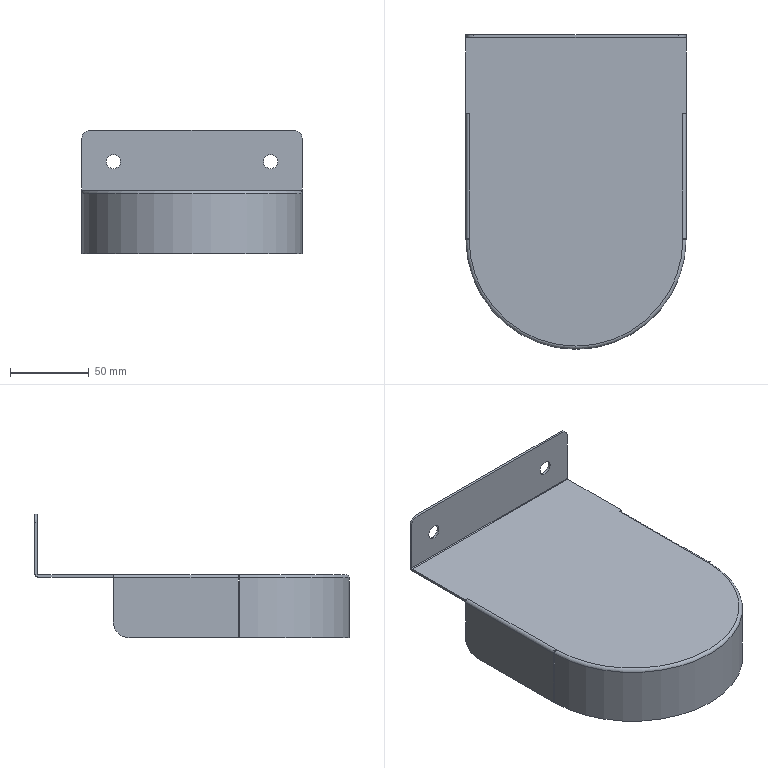Part | SolidWorks | features BaseBody 1 | 1 solid | 56 faces | box 140 x 200 x 78.5 mm | volume 67988 mm3 | plane 38 | cylinder 16 | torus 2 | commonest cylinder face diameters 9 x4 1 x3 4 x3 10 x2 20 x2 137 x1
STEP:
#1=CARTESIAN_POINT('',(-50.,128.5,23.));
#2=VERTEX_POINT('',#1);
#3=CARTESIAN_POINT('',(-50.,128.5,14.));
#4=VERTEX_POINT('',#3);
#5=CARTESIAN_POINT('',(-50.,128.5,18.5));
#6=DIRECTION('',(0.,-1.,0.));
#7=DIRECTION('',(0.,0.,-1.));
#8=AXIS2_PLACEMENT_3D('',#5,#6,#7);
#9=CIRCLE('',#8,4.5);
#10=EDGE_CURVE('',#2,#4,#9,.T.);
#11=ORIENTED_EDGE('',*,*,#10,.T.);
#12=CARTESIAN_POINT('',(-50.,130.,14.));
#13=VERTEX_POINT('',#12);
#14=CARTESIAN_POINT('',(-50.,120.,14.));
#15=DIRECTION('',(0.,1.,0.));
#16=VECTOR('',#15,1000.);
#17=LINE('',#14,#16);
#18=EDGE_CURVE('',#4,#13,#17,.T.);
#19=ORIENTED_EDGE('',*,*,#18,.T.);
#20=CARTESIAN_POINT('',(-50.,130.,23.));
#21=VERTEX_POINT('',#20);
#22=CARTESIAN_POINT('',(-50.,130.,18.5));
#23=DIRECTION('',(0.,1.,0.));
#24=DIRECTION('',(0.,0.,1.));
#25=AXIS2_PLACEMENT_3D('',#22,#23,#24);
#26=CIRCLE('',#25,4.5);
#27=EDGE_CURVE('',#13,#21,#26,.T.);
#28=ORIENTED_EDGE('',*,*,#27,.T.);
#29=CARTESIAN_POINT('',(-50.,120.,23.));
#30=DIRECTION('',(0.,1.,0.));
#31=VECTOR('',#30,1000.);
#32=LINE('',#29,#31);
#33=EDGE_CURVE('',#2,#21,#32,.T.);
#34=ORIENTED_EDGE('',*,*,#33,.F.);
#35=EDGE_LOOP('',(#11,#19,#28,#34));
#36=FACE_OUTER_BOUND('',#35,.T.);
#37=CARTESIAN_POINT('',(-50.,120.,18.5));
#38=DIRECTION('',(0.,1.,0.));
#39=DIRECTION('',(0.,0.,1.));
#40=AXIS2_PLACEMENT_3D('',#37,#38,#39);
#41=CYLINDRICAL_SURFACE('',#40,4.5);
#42=ADVANCED_FACE('',(#36),#41,.F.);
#43=CARTESIAN_POINT('',(50.,128.5,23.));
#44=VERTEX_POINT('',#43);
#45=CARTESIAN_POINT('',(50.,128.5,14.));
#46=VERTEX_POINT('',#45);
#47=CARTESIAN_POINT('',(50.,128.5,18.5));
#48=DIRECTION('',(0.,-1.,0.));
#49=DIRECTION('',(0.,0.,-1.));
#50=AXIS2_PLACEMENT_3D('',#47,#48,#49);
#51=CIRCLE('',#50,4.5);
#52=EDGE_CURVE('',#44,#46,#51,.T.);
#53=ORIENTED_EDGE('',*,*,#52,.T.);
#54=CARTESIAN_POINT('',(50.,130.,14.));
#55=VERTEX_POINT('',#54);
#56=CARTESIAN_POINT('',(50.,120.,14.));
#57=DIRECTION('',(0.,1.,0.));
#58=VECTOR('',#57,1000.);
#59=LINE('',#56,#58);
#60=EDGE_CURVE('',#46,#55,#59,.T.);
#61=ORIENTED_EDGE('',*,*,#60,.T.);
#62=CARTESIAN_POINT('',(50.,130.,23.));
#63=VERTEX_POINT('',#62);
#64=CARTESIAN_POINT('',(50.,130.,18.5));
#65=DIRECTION('',(0.,1.,0.));
#66=DIRECTION('',(0.,0.,1.));
#67=AXIS2_PLACEMENT_3D('',#64,#65,#66);
#68=CIRCLE('',#67,4.5);
#69=EDGE_CURVE('',#55,#63,#68,.T.);
#70=ORIENTED_EDGE('',*,*,#69,.T.);
#71=CARTESIAN_POINT('',(50.,120.,23.));
#72=DIRECTION('',(0.,1.,0.));
#73=VECTOR('',#72,1000.);
#74=LINE('',#71,#73);
#75=EDGE_CURVE('',#44,#63,#74,.T.);
#76=ORIENTED_EDGE('',*,*,#75,.F.);
#77=EDGE_LOOP('',(#53,#61,#70,#76));
#78=FACE_OUTER_BOUND('',#77,.T.);
#79=CARTESIAN_POINT('',(50.,120.,18.5));
#80=DIRECTION('',(0.,1.,0.));
#81=DIRECTION('',(0.,0.,1.));
#82=AXIS2_PLACEMENT_3D('',#79,#80,#81);
#83=CYLINDRICAL_SURFACE('',#82,4.5);
#84=ADVANCED_FACE('',(#78),#83,.F.);
#85=CARTESIAN_POINT('',(-70.,128.,-1.5));
#86=VERTEX_POINT('',#85);
#87=CARTESIAN_POINT('',(70.,128.,-1.5));
#88=VERTEX_POINT('',#87);
#89=CARTESIAN_POINT('',(-70.,128.,-1.5));
#90=DIRECTION('',(1.,0.,0.));
#91=VECTOR('',#90,1000.);
#92=LINE('',#89,#91);
#93=EDGE_CURVE('',#86,#88,#92,.T.);
#94=ORIENTED_EDGE('',*,*,#93,.T.);
#95=CARTESIAN_POINT('',(70.,80.,-1.5));
#96=VERTEX_POINT('',#95);
#97=CARTESIAN_POINT('',(70.,0.,-1.5));
#98=DIRECTION('',(0.,1.,0.));
#99=VECTOR('',#98,1000.);
#100=LINE('',#97,#99);
#101=EDGE_CURVE('',#96,#88,#100,.T.);
#102=ORIENTED_EDGE('',*,*,#101,.F.);
#103=CARTESIAN_POINT('',(69.936,80.,-1.5));
#104=VERTEX_POINT('',#103);
#105=CARTESIAN_POINT('',(68.,80.,-1.5));
#106=DIRECTION('',(1.,0.,0.));
#107=VECTOR('',#106,1000.);
#108=LINE('',#105,#107);
#109=EDGE_CURVE('',#104,#96,#108,.T.);
#110=ORIENTED_EDGE('',*,*,#109,.F.);
#111=CARTESIAN_POINT('',(68.,80.,-1.5));
#112=VERTEX_POINT('',#111);
#113=CARTESIAN_POINT('',(68.,80.,-1.5));
#114=DIRECTION('',(1.,0.,0.));
#115=VECTOR('',#114,1000.);
#116=LINE('',#113,#115);
#117=EDGE_CURVE('',#112,#104,#116,.T.);
#118=ORIENTED_EDGE('',*,*,#117,.F.);
#119=CARTESIAN_POINT('',(68.,0.5,-1.5));
#120=VERTEX_POINT('',#119);
#121=CARTESIAN_POINT('',(68.,0.5,-1.5));
#122=DIRECTION('',(0.,1.,0.));
#123=VECTOR('',#122,1000.);
#124=LINE('',#121,#123);
#125=EDGE_CURVE('',#120,#112,#124,.T.);
#126=ORIENTED_EDGE('',*,*,#125,.F.);
#127=CARTESIAN_POINT('',(69.936,0.5,-1.5));
#128=VERTEX_POINT('',#127);
#129=CARTESIAN_POINT('',(70.,0.5,-1.5));
#130=DIRECTION('',(-1.,0.,0.));
#131=VECTOR('',#130,1000.);
#132=LINE('',#129,#131);
#133=EDGE_CURVE('',#128,#120,#132,.T.);
#134=ORIENTED_EDGE('',*,*,#133,.F.);
#135=CARTESIAN_POINT('',(70.,0.5,-1.5));
#136=VERTEX_POINT('',#135);
#137=CARTESIAN_POINT('',(70.,0.5,-1.5));
#138=DIRECTION('',(-1.,0.,0.));
#139=VECTOR('',#138,1000.);
#140=LINE('',#137,#139);
#141=EDGE_CURVE('',#136,#128,#140,.T.);
#142=ORIENTED_EDGE('',*,*,#141,.F.);
#143=CARTESIAN_POINT('',(70.,0.,-1.5));
#144=VERTEX_POINT('',#143);
#145=CARTESIAN_POINT('',(70.,0.,-1.5));
#146=DIRECTION('',(0.,1.,0.));
#147=VECTOR('',#146,1000.);
#148=LINE('',#145,#147);
#149=EDGE_CURVE('',#144,#136,#148,.T.);
#150=ORIENTED_EDGE('',*,*,#149,.F.);
#151=CARTESIAN_POINT('',(69.936,0.,-1.5));
#152=VERTEX_POINT('',#151);
#153=CARTESIAN_POINT('',(68.,0.,-1.5));
#154=DIRECTION('',(1.,0.,0.));
#155=VECTOR('',#154,1000.);
#156=LINE('',#153,#155);
#157=EDGE_CURVE('',#152,#144,#156,.T.);
#158=ORIENTED_EDGE('',*,*,#157,.F.);
#159=CARTESIAN_POINT('',(68.,0.,-1.5));
#160=VERTEX_POINT('',#159);
#161=CARTESIAN_POINT('',(68.,0.,-1.5));
#162=DIRECTION('',(1.,0.,0.));
#163=VECTOR('',#162,1000.);
#164=LINE('',#161,#163);
#165=EDGE_CURVE('',#160,#152,#164,.T.);
#166=ORIENTED_EDGE('',*,*,#165,.F.);
#167=CARTESIAN_POINT('',(-68.,0.,-1.5));
#168=VERTEX_POINT('',#167);
#169=CARTESIAN_POINT('',(0.,0.,-1.5));
#170=DIRECTION('',(0.,0.,1.));
#171=DIRECTION('',(-1.,0.,0.));
#172=AXIS2_PLACEMENT_3D('',#169,#170,#171);
#173=CIRCLE('',#172,68.);
#174=EDGE_CURVE('',#168,#160,#173,.T.);
#175=ORIENTED_EDGE('',*,*,#174,.F.);
#176=CARTESIAN_POINT('',(-69.936,0.,-1.5));
#177=VERTEX_POINT('',#176);
#178=CARTESIAN_POINT('',(-70.,0.,-1.5));
#179=DIRECTION('',(1.,0.,0.));
#180=VECTOR('',#179,1000.);
#181=LINE('',#178,#180);
#182=EDGE_CURVE('',#177,#168,#181,.T.);
#183=ORIENTED_EDGE('',*,*,#182,.F.);
#184=CARTESIAN_POINT('',(-70.,0.,-1.5));
#185=VERTEX_POINT('',#184);
#186=CARTESIAN_POINT('',(-70.,0.,-1.5));
#187=DIRECTION('',(1.,0.,0.));
#188=VECTOR('',#187,1000.);
#189=LINE('',#186,#188);
#190=EDGE_CURVE('',#185,#177,#189,.T.);
#191=ORIENTED_EDGE('',*,*,#190,.F.);
#192=CARTESIAN_POINT('',(-70.,0.5,-1.5));
#193=VERTEX_POINT('',#192);
#194=CARTESIAN_POINT('',(-70.,0.,-1.5));
#195=DIRECTION('',(0.,-1.,0.));
#196=VECTOR('',#195,1000.);
#197=LINE('',#194,#196);
#198=EDGE_CURVE('',#193,#185,#197,.T.);
#199=ORIENTED_EDGE('',*,*,#198,.F.);
#200=CARTESIAN_POINT('',(-69.936,0.5,-1.5));
#201=VERTEX_POINT('',#200);
#202=CARTESIAN_POINT('',(-68.,0.5,-1.5));
#203=DIRECTION('',(-1.,0.,0.));
#204=VECTOR('',#203,1000.);
#205=LINE('',#202,#204);
#206=EDGE_CURVE('',#201,#193,#205,.T.);
#207=ORIENTED_EDGE('',*,*,#206,.F.);
#208=CARTESIAN_POINT('',(-68.,0.5,-1.5));
#209=VERTEX_POINT('',#208);
#210=CARTESIAN_POINT('',(-68.,0.5,-1.5));
#211=DIRECTION('',(-1.,0.,0.));
#212=VECTOR('',#211,1000.);
#213=LINE('',#210,#212);
#214=EDGE_CURVE('',#209,#201,#213,.T.);
#215=ORIENTED_EDGE('',*,*,#214,.F.);
#216=CARTESIAN_POINT('',(-68.,80.,-1.5));
#217=VERTEX_POINT('',#216);
#218=CARTESIAN_POINT('',(-68.,80.,-1.5));
#219=DIRECTION('',(0.,-1.,0.));
#220=VECTOR('',#219,1000.);
#221=LINE('',#218,#220);
#222=EDGE_CURVE('',#217,#209,#221,.T.);
#223=ORIENTED_EDGE('',*,*,#222,.F.);
#224=CARTESIAN_POINT('',(-69.936,80.,-1.5));
#225=VERTEX_POINT('',#224);
#226=CARTESIAN_POINT('',(-70.,80.,-1.5));
#227=DIRECTION('',(1.,0.,0.));
#228=VECTOR('',#227,1000.);
#229=LINE('',#226,#228);
#230=EDGE_CURVE('',#225,#217,#229,.T.);
#231=ORIENTED_EDGE('',*,*,#230,.F.);
#232=CARTESIAN_POINT('',(-70.,80.,-1.5));
#233=VERTEX_POINT('',#232);
#234=CARTESIAN_POINT('',(-70.,80.,-1.5));
#235=DIRECTION('',(1.,0.,0.));
#236=VECTOR('',#235,1000.);
#237=LINE('',#234,#236);
#238=EDGE_CURVE('',#233,#225,#237,.T.);
#239=ORIENTED_EDGE('',*,*,#238,.F.);
#240=CARTESIAN_POINT('',(-70.,0.,-1.5));
#241=DIRECTION('',(0.,-1.,0.));
#242=VECTOR('',#241,1000.);
#243=LINE('',#240,#242);
#244=EDGE_CURVE('',#86,#233,#243,.T.);
#245=ORIENTED_EDGE('',*,*,#244,.F.);
#246=EDGE_LOOP('',(#94,#102,#110,#118,#126,#134,#142,#150,#158,#166,#175,#183,#191,#199,#207,#215,#223,#231,#239,#245));
#247=FACE_OUTER_BOUND('',#246,.T.);
#248=CARTESIAN_POINT('',(0.,0.,-1.5));
#249=DIRECTION('',(0.,0.,1.));
#250=DIRECTION('',(1.,0.,0.));
#251=AXIS2_PLACEMENT_3D('',#248,#249,#250);
#252=PLANE('',#251);
#253=ADVANCED_FACE('',(#247),#252,.F.);
#254=CARTESIAN_POINT('',(70.,80.,0.));
#255=VERTEX_POINT('',#254);
#256=CARTESIAN_POINT('',(70.,128.,0.));
#257=VERTEX_POINT('',#256);
#258=CARTESIAN_POINT('',(70.,0.,0.));
#259=DIRECTION('',(0.,1.,0.));
#260=VECTOR('',#259,1000.);
#261=LINE('',#258,#260);
#262=EDGE_CURVE('',#255,#257,#261,.T.);
#263=ORIENTED_EDGE('',*,*,#262,.T.);
#264=CARTESIAN_POINT('',(-70.,128.,0.));
#265=VERTEX_POINT('',#264);
#266=CARTESIAN_POINT('',(-70.,128.,0.));
#267=DIRECTION('',(1.,0.,0.));
#268=VECTOR('',#267,1000.);
#269=LINE('',#266,#268);
#270=EDGE_CURVE('',#265,#257,#269,.T.);
#271=ORIENTED_EDGE('',*,*,#270,.F.);
#272=CARTESIAN_POINT('',(-70.,80.,0.));
#273=VERTEX_POINT('',#272);
#274=CARTESIAN_POINT('',(-70.,0.,0.));
#275=DIRECTION('',(0.,-1.,0.));
#276=VECTOR('',#275,1000.);
#277=LINE('',#274,#276);
#278=EDGE_CURVE('',#265,#273,#277,.T.);
#279=ORIENTED_EDGE('',*,*,#278,.T.);
#280=CARTESIAN_POINT('',(-68.,80.,0.));
#281=VERTEX_POINT('',#280);
#282=CARTESIAN_POINT('',(0.,80.,0.));
#283=DIRECTION('',(1.,0.,0.));
#284=VECTOR('',#283,1000.);
#285=LINE('',#282,#284);
#286=EDGE_CURVE('',#273,#281,#285,.T.);
#287=ORIENTED_EDGE('',*,*,#286,.T.);
#288=CARTESIAN_POINT('',(-68.,0.5,0.));
#289=VERTEX_POINT('',#288);
#290=CARTESIAN_POINT('',(-68.,80.,0.));
#291=DIRECTION('',(0.,-1.,0.));
#292=VECTOR('',#291,1000.);
#293=LINE('',#290,#292);
#294=EDGE_CURVE('',#281,#289,#293,.T.);
#295=ORIENTED_EDGE('',*,*,#294,.T.);
#296=CARTESIAN_POINT('',(-70.,0.5,0.));
#297=VERTEX_POINT('',#296);
#298=CARTESIAN_POINT('',(0.,0.5,0.));
#299=DIRECTION('',(-1.,0.,0.));
#300=VECTOR('',#299,1000.);
#301=LINE('',#298,#300);
#302=EDGE_CURVE('',#289,#297,#301,.T.);
#303=ORIENTED_EDGE('',*,*,#302,.T.);
#304=CARTESIAN_POINT('',(-70.,0.,0.));
#305=VERTEX_POINT('',#304);
#306=CARTESIAN_POINT('',(-70.,0.,0.));
#307=DIRECTION('',(0.,-1.,0.));
#308=VECTOR('',#307,1000.);
#309=LINE('',#306,#308);
#310=EDGE_CURVE('',#297,#305,#309,.T.);
#311=ORIENTED_EDGE('',*,*,#310,.T.);
#312=CARTESIAN_POINT('',(-68.,0.,0.));
#313=VERTEX_POINT('',#312);
#314=CARTESIAN_POINT('',(0.,0.,0.));
#315=DIRECTION('',(1.,0.,0.));
#316=VECTOR('',#315,1000.);
#317=LINE('',#314,#316);
#318=EDGE_CURVE('',#305,#313,#317,.T.);
#319=ORIENTED_EDGE('',*,*,#318,.T.);
#320=CARTESIAN_POINT('',(68.,0.,0.));
#321=VERTEX_POINT('',#320);
#322=CARTESIAN_POINT('',(0.,0.,0.));
#323=DIRECTION('',(0.,0.,1.));
#324=DIRECTION('',(1.,0.,0.));
#325=AXIS2_PLACEMENT_3D('',#322,#323,#324);
#326=CIRCLE('',#325,68.);
#327=EDGE_CURVE('',#313,#321,#326,.T.);
#328=ORIENTED_EDGE('',*,*,#327,.T.);
#329=CARTESIAN_POINT('',(70.,0.,0.));
#330=VERTEX_POINT('',#329);
#331=CARTESIAN_POINT('',(0.,0.,0.));
#332=DIRECTION('',(1.,0.,0.));
#333=VECTOR('',#332,1000.);
#334=LINE('',#331,#333);
#335=EDGE_CURVE('',#321,#330,#334,.T.);
#336=ORIENTED_EDGE('',*,*,#335,.T.);
#337=CARTESIAN_POINT('',(70.,0.5,0.));
#338=VERTEX_POINT('',#337);
#339=CARTESIAN_POINT('',(70.,0.,0.));
#340=DIRECTION('',(0.,1.,0.));
#341=VECTOR('',#340,1000.);
#342=LINE('',#339,#341);
#343=EDGE_CURVE('',#330,#338,#342,.T.);
#344=ORIENTED_EDGE('',*,*,#343,.T.);
#345=CARTESIAN_POINT('',(68.,0.5,0.));
#346=VERTEX_POINT('',#345);
#347=CARTESIAN_POINT('',(0.,0.5,0.));
#348=DIRECTION('',(-1.,0.,0.));
#349=VECTOR('',#348,1000.);
#350=LINE('',#347,#349);
#351=EDGE_CURVE('',#338,#346,#350,.T.);
#352=ORIENTED_EDGE('',*,*,#351,.T.);
#353=CARTESIAN_POINT('',(68.,80.,0.));
#354=VERTEX_POINT('',#353);
#355=CARTESIAN_POINT('',(68.,0.5,0.));
#356=DIRECTION('',(0.,1.,0.));
#357=VECTOR('',#356,1000.);
#358=LINE('',#355,#357);
#359=EDGE_CURVE('',#346,#354,#358,.T.);
#360=ORIENTED_EDGE('',*,*,#359,.T.);
#361=CARTESIAN_POINT('',(0.,80.,0.));
#362=DIRECTION('',(1.,0.,0.));
#363=VECTOR('',#362,1000.);
#364=LINE('',#361,#363);
#365=EDGE_CURVE('',#354,#255,#364,.T.);
#366=ORIENTED_EDGE('',*,*,#365,.T.);
#367=EDGE_LOOP('',(#263,#271,#279,#287,#295,#303,#311,#319,#328,#336,#344,#352,#360,#366));
#368=FACE_OUTER_BOUND('',#367,.T.);
#369=CARTESIAN_POINT('',(0.,0.,0.));
#370=DIRECTION('',(0.,0.,1.));
#371=DIRECTION('',(1.,0.,0.));
#372=AXIS2_PLACEMENT_3D('',#369,#370,#371);
#373=PLANE('',#372);
#374=ADVANCED_FACE('',(#368),#373,.T.);
#375=ORIENTED_EDGE('',*,*,#278,.F.);
#376=CARTESIAN_POINT('',(-70.,128.,0.));
#377=DIRECTION('',(0.,0.,-1.));
#378=VECTOR('',#377,1000.);
#379=LINE('',#376,#378);
#380=EDGE_CURVE('',#265,#86,#379,.T.);
#381=ORIENTED_EDGE('',*,*,#380,.T.);
#382=ORIENTED_EDGE('',*,*,#244,.T.);
#383=CARTESIAN_POINT('',(-70.,80.,-1.5));
#384=DIRECTION('',(0.,0.,1.));
#385=VECTOR('',#384,1000.);
#386=LINE('',#383,#385);
#387=EDGE_CURVE('',#233,#273,#386,.T.);
#388=ORIENTED_EDGE('',*,*,#387,.T.);
#389=EDGE_LOOP('',(#375,#381,#382,#388));
#390=FACE_OUTER_BOUND('',#389,.T.);
#391=CARTESIAN_POINT('',(-70.,0.,-1.5));
#392=DIRECTION('',(-1.,0.,0.));
#393=DIRECTION('',(0.,-1.,0.));
#394=AXIS2_PLACEMENT_3D('',#391,#392,#393);
#395=PLANE('',#394);
#396=ADVANCED_FACE('',(#390),#395,.T.);
#397=ORIENTED_EDGE('',*,*,#365,.F.);
#398=CARTESIAN_POINT('',(68.,80.,-2.));
#399=DIRECTION('',(0.,1.,0.));
#400=DIRECTION('',(0.,0.,-1.));
#401=AXIS2_PLACEMENT_3D('',#398,#399,#400);
#402=CIRCLE('',#401,2.);
#403=EDGE_CURVE('',#354,#104,#402,.T.);
#404=ORIENTED_EDGE('',*,*,#403,.T.);
#405=ORIENTED_EDGE('',*,*,#109,.T.);
#406=CARTESIAN_POINT('',(70.,80.,-1.5));
#407=DIRECTION('',(0.,0.,1.));
#408=VECTOR('',#407,1000.);
#409=LINE('',#406,#408);
#410=EDGE_CURVE('',#96,#255,#409,.T.);
#411=ORIENTED_EDGE('',*,*,#410,.T.);
#412=EDGE_LOOP('',(#397,#404,#405,#411));
#413=FACE_OUTER_BOUND('',#412,.T.);
#414=CARTESIAN_POINT('',(68.,80.,-1.5));
#415=DIRECTION('',(0.,-1.,0.));
#416=DIRECTION('',(0.,0.,-1.));
#417=AXIS2_PLACEMENT_3D('',#414,#415,#416);
#418=PLANE('',#417);
#419=ADVANCED_FACE('',(#413),#418,.T.);
#420=ORIENTED_EDGE('',*,*,#141,.T.);
#421=CARTESIAN_POINT('',(68.,0.5,-2.));
#422=DIRECTION('',(0.,-1.,0.));
#423=DIRECTION('',(0.,0.,-1.));
#424=AXIS2_PLACEMENT_3D('',#421,#422,#423);
#425=CIRCLE('',#424,2.);
#426=EDGE_CURVE('',#128,#346,#425,.T.);
#427=ORIENTED_EDGE('',*,*,#426,.T.);
#428=ORIENTED_EDGE('',*,*,#351,.F.);
#429=CARTESIAN_POINT('',(70.,0.5,-1.5));
#430=DIRECTION('',(0.,0.,1.));
#431=VECTOR('',#430,1000.);
#432=LINE('',#429,#431);
#433=EDGE_CURVE('',#136,#338,#432,.T.);
#434=ORIENTED_EDGE('',*,*,#433,.F.);
#435=EDGE_LOOP('',(#420,#427,#428,#434));
#436=FACE_OUTER_BOUND('',#435,.T.);
#437=CARTESIAN_POINT('',(70.,0.5,-1.5));
#438=DIRECTION('',(0.,1.,0.));
#439=DIRECTION('',(-1.,0.,0.));
#440=AXIS2_PLACEMENT_3D('',#437,#438,#439);
#441=PLANE('',#440);
#442=ADVANCED_FACE('',(#436),#441,.T.);
#443=ORIENTED_EDGE('',*,*,#238,.T.);
#444=CARTESIAN_POINT('',(-68.,80.,-2.));
#445=DIRECTION('',(0.,1.,0.));
#446=DIRECTION('',(0.,0.,1.));
#447=AXIS2_PLACEMENT_3D('',#444,#445,#446);
#448=CIRCLE('',#447,2.);
#449=EDGE_CURVE('',#225,#281,#448,.T.);
#450=ORIENTED_EDGE('',*,*,#449,.T.);
#451=ORIENTED_EDGE('',*,*,#286,.F.);
#452=ORIENTED_EDGE('',*,*,#387,.F.);
#453=EDGE_LOOP('',(#443,#450,#451,#452));
#454=FACE_OUTER_BOUND('',#453,.T.);
#455=CARTESIAN_POINT('',(-70.,80.,-1.5));
#456=DIRECTION('',(0.,-1.,0.));
#457=DIRECTION('',(0.,0.,-1.));
#458=AXIS2_PLACEMENT_3D('',#455,#456,#457);
#459=PLANE('',#458);
#460=ADVANCED_FACE('',(#454),#459,.T.);
#461=ORIENTED_EDGE('',*,*,#302,.F.);
#462=CARTESIAN_POINT('',(-68.,0.5,-2.));
#463=DIRECTION('',(0.,-1.,0.));
#464=DIRECTION('',(0.,0.,1.));
#465=AXIS2_PLACEMENT_3D('',#462,#463,#464);
#466=CIRCLE('',#465,2.);
#467=EDGE_CURVE('',#289,#201,#466,.T.);
#468=ORIENTED_EDGE('',*,*,#467,.T.);
#469=ORIENTED_EDGE('',*,*,#206,.T.);
#470=CARTESIAN_POINT('',(-70.,0.5,-1.5));
#471=DIRECTION('',(0.,0.,1.));
#472=VECTOR('',#471,1000.);
#473=LINE('',#470,#472);
#474=EDGE_CURVE('',#193,#297,#473,.T.);
#475=ORIENTED_EDGE('',*,*,#474,.T.);
#476=EDGE_LOOP('',(#461,#468,#469,#475));
#477=FACE_OUTER_BOUND('',#476,.T.);
#478=CARTESIAN_POINT('',(-68.,0.5,-1.5));
#479=DIRECTION('',(0.,1.,0.));
#480=DIRECTION('',(-1.,0.,0.));
#481=AXIS2_PLACEMENT_3D('',#478,#479,#480);
#482=PLANE('',#481);
#483=ADVANCED_FACE('',(#477),#482,.T.);
#484=ORIENTED_EDGE('',*,*,#149,.T.);
#485=ORIENTED_EDGE('',*,*,#433,.T.);
#486=ORIENTED_EDGE('',*,*,#343,.F.);
#487=CARTESIAN_POINT('',(70.,0.,-1.5));
#488=DIRECTION('',(0.,0.,1.));
#489=VECTOR('',#488,1000.);
#490=LINE('',#487,#489);
#491=EDGE_CURVE('',#144,#330,#490,.T.);
#492=ORIENTED_EDGE('',*,*,#491,.F.);
#493=EDGE_LOOP('',(#484,#485,#486,#492));
#494=FACE_OUTER_BOUND('',#493,.T.);
#495=CARTESIAN_POINT('',(70.,0.,-1.5));
#496=DIRECTION('',(1.,0.,0.));
#497=DIRECTION('',(0.,1.,0.));
#498=AXIS2_PLACEMENT_3D('',#495,#496,#497);
#499=PLANE('',#498);
#500=ADVANCED_FACE('',(#494),#499,.T.);
#501=CARTESIAN_POINT('',(70.,128.,0.));
#502=DIRECTION('',(0.,0.,-1.));
#503=VECTOR('',#502,1000.);
#504=LINE('',#501,#503);
#505=EDGE_CURVE('',#257,#88,#504,.T.);
#506=ORIENTED_EDGE('',*,*,#505,.F.);
#507=ORIENTED_EDGE('',*,*,#262,.F.);
#508=ORIENTED_EDGE('',*,*,#410,.F.);
#509=ORIENTED_EDGE('',*,*,#101,.T.);
#510=EDGE_LOOP('',(#506,#507,#508,#509));
#511=FACE_OUTER_BOUND('',#510,.T.);
#512=CARTESIAN_POINT('',(70.,0.,-1.5));
#513=DIRECTION('',(1.,0.,0.));
#514=DIRECTION('',(0.,1.,0.));
#515=AXIS2_PLACEMENT_3D('',#512,#513,#514);
#516=PLANE('',#515);
#517=ADVANCED_FACE('',(#511),#516,.T.);
#518=ORIENTED_EDGE('',*,*,#310,.F.);
#519=ORIENTED_EDGE('',*,*,#474,.F.);
#520=ORIENTED_EDGE('',*,*,#198,.T.);
#521=CARTESIAN_POINT('',(-70.,0.,-1.5));
#522=DIRECTION('',(0.,0.,1.));
#523=VECTOR('',#522,1000.);
#524=LINE('',#521,#523);
#525=EDGE_CURVE('',#185,#305,#524,.T.);
#526=ORIENTED_EDGE('',*,*,#525,.T.);
#527=EDGE_LOOP('',(#518,#519,#520,#526));
#528=FACE_OUTER_BOUND('',#527,.T.);
#529=CARTESIAN_POINT('',(-70.,0.,-1.5));
#530=DIRECTION('',(-1.,0.,0.));
#531=DIRECTION('',(0.,-1.,0.));
#532=AXIS2_PLACEMENT_3D('',#529,#530,#531);
#533=PLANE('',#532);
#534=ADVANCED_FACE('',(#528),#533,.T.);
#535=ORIENTED_EDGE('',*,*,#335,.F.);
#536=CARTESIAN_POINT('',(68.,0.,-2.));
#537=DIRECTION('',(0.,1.,0.));
#538=DIRECTION('',(1.,0.,0.));
#539=AXIS2_PLACEMENT_3D('',#536,#537,#538);
#540=CIRCLE('',#539,2.);
#541=EDGE_CURVE('',#321,#152,#540,.T.);
#542=ORIENTED_EDGE('',*,*,#541,.T.);
#543=ORIENTED_EDGE('',*,*,#157,.T.);
#544=ORIENTED_EDGE('',*,*,#491,.T.);
#545=EDGE_LOOP('',(#535,#542,#543,#544));
#546=FACE_OUTER_BOUND('',#545,.T.);
#547=CARTESIAN_POINT('',(68.,0.,-1.5));
#548=DIRECTION('',(0.,-1.,0.));
#549=DIRECTION('',(1.,0.,0.));
#550=AXIS2_PLACEMENT_3D('',#547,#548,#549);
#551=PLANE('',#550);
#552=ADVANCED_FACE('',(#546),#551,.T.);
#553=CARTESIAN_POINT('',(-68.,0.,-2.));
#554=DIRECTION('',(0.,-1.,0.));
#555=DIRECTION('',(-1.,0.,0.));
#556=AXIS2_PLACEMENT_3D('',#553,#554,#555);
#557=CIRCLE('',#556,2.);
#558=EDGE_CURVE('',#313,#177,#557,.T.);
#559=ORIENTED_EDGE('',*,*,#558,.F.);
#560=ORIENTED_EDGE('',*,*,#318,.F.);
#561=ORIENTED_EDGE('',*,*,#525,.F.);
#562=ORIENTED_EDGE('',*,*,#190,.T.);
#563=EDGE_LOOP('',(#559,#560,#561,#562));
#564=FACE_OUTER_BOUND('',#563,.T.);
#565=CARTESIAN_POINT('',(-70.,0.,-1.5));
#566=DIRECTION('',(0.,-1.,0.));
#567=DIRECTION('',(1.,0.,0.));
#568=AXIS2_PLACEMENT_3D('',#565,#566,#567);
#569=PLANE('',#568);
#570=ADVANCED_FACE('',(#564),#569,.T.);
#571=CARTESIAN_POINT('',(68.5,0.,-2.));
#572=VERTEX_POINT('',#571);
#573=CARTESIAN_POINT('',(68.,0.,-2.));
#574=DIRECTION('',(0.,1.,0.));
#575=DIRECTION('',(0.,0.,-1.));
#576=AXIS2_PLACEMENT_3D('',#573,#574,#575);
#577=CIRCLE('',#576,0.5);
#578=EDGE_CURVE('',#160,#572,#577,.T.);
#579=ORIENTED_EDGE('',*,*,#578,.F.);
#580=ORIENTED_EDGE('',*,*,#165,.T.);
#581=CARTESIAN_POINT('',(70.,0.,-2.));
#582=VERTEX_POINT('',#581);
#583=CARTESIAN_POINT('',(68.,0.,-2.));
#584=DIRECTION('',(0.,1.,0.));
#585=DIRECTION('',(1.,0.,0.));
#586=AXIS2_PLACEMENT_3D('',#583,#584,#585);
#587=CIRCLE('',#586,2.);
#588=EDGE_CURVE('',#152,#582,#587,.T.);
#589=ORIENTED_EDGE('',*,*,#588,.T.);
#590=CARTESIAN_POINT('',(68.5,0.,-2.));
#591=DIRECTION('',(1.,0.,0.));
#592=VECTOR('',#591,1000.);
#593=LINE('',#590,#592);
#594=EDGE_CURVE('',#572,#582,#593,.T.);
#595=ORIENTED_EDGE('',*,*,#594,.F.);
#596=EDGE_LOOP('',(#579,#580,#589,#595));
#597=FACE_OUTER_BOUND('',#596,.T.);
#598=CARTESIAN_POINT('',(68.,0.,-2.));
#599=DIRECTION('',(0.,1.,0.));
#600=DIRECTION('',(0.,0.,1.));
#601=AXIS2_PLACEMENT_3D('',#598,#599,#600);
#602=PLANE('',#601);
#603=ADVANCED_FACE('',(#597),#602,.T.);
#604=CARTESIAN_POINT('',(-70.,0.,-2.));
#605=VERTEX_POINT('',#604);
#606=CARTESIAN_POINT('',(-68.,0.,-2.));
#607=DIRECTION('',(0.,-1.,0.));
#608=DIRECTION('',(-1.,0.,0.));
#609=AXIS2_PLACEMENT_3D('',#606,#607,#608);
#610=CIRCLE('',#609,2.);
#611=EDGE_CURVE('',#177,#605,#610,.T.);
#612=ORIENTED_EDGE('',*,*,#611,.F.);
#613=ORIENTED_EDGE('',*,*,#182,.T.);
#614=CARTESIAN_POINT('',(-68.5,0.,-2.));
#615=VERTEX_POINT('',#614);
#616=CARTESIAN_POINT('',(-68.,0.,-2.));
#617=DIRECTION('',(0.,-1.,0.));
#618=DIRECTION('',(0.,0.,-1.));
#619=AXIS2_PLACEMENT_3D('',#616,#617,#618);
#620=CIRCLE('',#619,0.5);
#621=EDGE_CURVE('',#168,#615,#620,.T.);
#622=ORIENTED_EDGE('',*,*,#621,.T.);
#623=CARTESIAN_POINT('',(-68.5,0.,-2.));
#624=DIRECTION('',(-1.,0.,0.));
#625=VECTOR('',#624,1000.);
#626=LINE('',#623,#625);
#627=EDGE_CURVE('',#615,#605,#626,.T.);
#628=ORIENTED_EDGE('',*,*,#627,.T.);
#629=EDGE_LOOP('',(#612,#613,#622,#628));
#630=FACE_OUTER_BOUND('',#629,.T.);
#631=CARTESIAN_POINT('',(-68.,0.,-2.));
#632=DIRECTION('',(0.,-1.,0.));
#633=DIRECTION('',(1.,0.,0.));
#634=AXIS2_PLACEMENT_3D('',#631,#632,#633);
#635=PLANE('',#634);
#636=ADVANCED_FACE('',(#630),#635,.F.);
#637=ORIENTED_EDGE('',*,*,#627,.F.);
#638=CARTESIAN_POINT('',(-68.5,0.,-40.));
#639=VERTEX_POINT('',#638);
#640=CARTESIAN_POINT('',(-68.5,0.,-1.5));
#641=DIRECTION('',(0.,0.,-1.));
#642=VECTOR('',#641,1000.);
#643=LINE('',#640,#642);
#644=EDGE_CURVE('',#615,#639,#643,.T.);
#645=ORIENTED_EDGE('',*,*,#644,.T.);
#646=CARTESIAN_POINT('',(-70.,0.,-40.));
#647=VERTEX_POINT('',#646);
#648=CARTESIAN_POINT('',(-68.5,0.,-40.));
#649=DIRECTION('',(-1.,0.,0.));
#650=VECTOR('',#649,1000.);
#651=LINE('',#648,#650);
#652=EDGE_CURVE('',#639,#647,#651,.T.);
#653=ORIENTED_EDGE('',*,*,#652,.T.);
#654=CARTESIAN_POINT('',(-70.,0.,-1.5));
#655=DIRECTION('',(0.,0.,-1.));
#656=VECTOR('',#655,1000.);
#657=LINE('',#654,#656);
#658=EDGE_CURVE('',#605,#647,#657,.T.);
#659=ORIENTED_EDGE('',*,*,#658,.F.);
#660=EDGE_LOOP('',(#637,#645,#653,#659));
#661=FACE_OUTER_BOUND('',#660,.T.);
#662=CARTESIAN_POINT('',(-68.5,0.,-21.));
#663=DIRECTION('',(0.,1.,0.));
#664=DIRECTION('',(0.,0.,-1.));
#665=AXIS2_PLACEMENT_3D('',#662,#663,#664);
#666=PLANE('',#665);
#667=ADVANCED_FACE('',(#661),#666,.T.);
#668=ORIENTED_EDGE('',*,*,#652,.F.);
#669=CARTESIAN_POINT('',(68.5,0.,-40.));
#670=VERTEX_POINT('',#669);
#671=CARTESIAN_POINT('',(0.,0.,-40.));
#672=DIRECTION('',(0.,0.,1.));
#673=DIRECTION('',(-1.,0.,0.));
#674=AXIS2_PLACEMENT_3D('',#671,#672,#673);
#675=CIRCLE('',#674,68.5);
#676=EDGE_CURVE('',#639,#670,#675,.T.);
#677=ORIENTED_EDGE('',*,*,#676,.T.);
#678=CARTESIAN_POINT('',(70.,0.,-40.));
#679=VERTEX_POINT('',#678);
#680=CARTESIAN_POINT('',(68.5,0.,-40.));
#681=DIRECTION('',(1.,0.,0.));
#682=VECTOR('',#681,1000.);
#683=LINE('',#680,#682);
#684=EDGE_CURVE('',#670,#679,#683,.T.);
#685=ORIENTED_EDGE('',*,*,#684,.T.);
#686=CARTESIAN_POINT('',(0.,0.,-40.));
#687=DIRECTION('',(0.,0.,1.));
#688=DIRECTION('',(1.,0.,0.));
#689=AXIS2_PLACEMENT_3D('',#686,#687,#688);
#690=CIRCLE('',#689,70.);
#691=EDGE_CURVE('',#647,#679,#690,.T.);
#692=ORIENTED_EDGE('',*,*,#691,.F.);
#693=EDGE_LOOP('',(#668,#677,#685,#692));
#694=FACE_OUTER_BOUND('',#693,.T.);
#695=CARTESIAN_POINT('',(0.,0.,-40.));
#696=DIRECTION('',(0.,0.,-1.));
#697=DIRECTION('',(-1.,0.,0.));
#698=AXIS2_PLACEMENT_3D('',#695,#696,#697);
#699=PLANE('',#698);
#700=ADVANCED_FACE('',(#694),#699,.T.);
#701=CARTESIAN_POINT('',(68.5,0.,-1.5));
#702=DIRECTION('',(0.,0.,-1.));
#703=VECTOR('',#702,1000.);
#704=LINE('',#701,#703);
#705=EDGE_CURVE('',#572,#670,#704,.T.);
#706=ORIENTED_EDGE('',*,*,#705,.F.);
#707=ORIENTED_EDGE('',*,*,#594,.T.);
#708=CARTESIAN_POINT('',(70.,0.,-1.5));
#709=DIRECTION('',(0.,0.,-1.));
#710=VECTOR('',#709,1000.);
#711=LINE('',#708,#710);
#712=EDGE_CURVE('',#582,#679,#711,.T.);
#713=ORIENTED_EDGE('',*,*,#712,.T.);
#714=ORIENTED_EDGE('',*,*,#684,.F.);
#715=EDGE_LOOP('',(#706,#707,#713,#714));
#716=FACE_OUTER_BOUND('',#715,.T.);
#717=CARTESIAN_POINT('',(68.5,0.,-21.));
#718=DIRECTION('',(0.,-1.,0.));
#719=DIRECTION('',(0.,0.,-1.));
#720=AXIS2_PLACEMENT_3D('',#717,#718,#719);
#721=PLANE('',#720);
#722=ADVANCED_FACE('',(#716),#721,.F.);
#723=ORIENTED_EDGE('',*,*,#691,.T.);
#724=ORIENTED_EDGE('',*,*,#712,.F.);
#725=CARTESIAN_POINT('',(0.,0.,-2.));
#726=DIRECTION('',(0.,0.,1.));
#727=DIRECTION('',(1.,0.,0.));
#728=AXIS2_PLACEMENT_3D('',#725,#726,#727);
#729=CIRCLE('',#728,70.);
#730=EDGE_CURVE('',#605,#582,#729,.T.);
#731=ORIENTED_EDGE('',*,*,#730,.F.);
#732=ORIENTED_EDGE('',*,*,#658,.T.);
#733=EDGE_LOOP('',(#723,#724,#731,#732));
#734=FACE_OUTER_BOUND('',#733,.T.);
#735=CARTESIAN_POINT('',(0.,0.,-1.5));
#736=DIRECTION('',(0.,0.,1.));
#737=DIRECTION('',(1.,0.,0.));
#738=AXIS2_PLACEMENT_3D('',#735,#736,#737);
#739=CYLINDRICAL_SURFACE('',#738,70.);
#740=ADVANCED_FACE('',(#734),#739,.T.);
#741=ORIENTED_EDGE('',*,*,#730,.T.);
#742=ORIENTED_EDGE('',*,*,#588,.F.);
#743=ORIENTED_EDGE('',*,*,#541,.F.);
#744=ORIENTED_EDGE('',*,*,#327,.F.);
#745=ORIENTED_EDGE('',*,*,#558,.T.);
#746=ORIENTED_EDGE('',*,*,#611,.T.);
#747=EDGE_LOOP('',(#741,#742,#743,#744,#745,#746));
#748=FACE_OUTER_BOUND('',#747,.T.);
#749=CARTESIAN_POINT('',(0.,0.,-2.));
#750=DIRECTION('',(0.,0.,1.));
#751=DIRECTION('',(1.,0.,0.));
#752=AXIS2_PLACEMENT_3D('',#749,#750,#751);
#753=TOROIDAL_SURFACE('',#752,68.,2.);
#754=ADVANCED_FACE('',(#748),#753,.T.);
#755=ORIENTED_EDGE('',*,*,#676,.F.);
#756=ORIENTED_EDGE('',*,*,#644,.F.);
#757=CARTESIAN_POINT('',(0.,0.,-2.));
#758=DIRECTION('',(0.,0.,1.));
#759=DIRECTION('',(-1.,0.,0.));
#760=AXIS2_PLACEMENT_3D('',#757,#758,#759);
#761=CIRCLE('',#760,68.5);
#762=EDGE_CURVE('',#615,#572,#761,.T.);
#763=ORIENTED_EDGE('',*,*,#762,.T.);
#764=ORIENTED_EDGE('',*,*,#705,.T.);
#765=EDGE_LOOP('',(#755,#756,#763,#764));
#766=FACE_OUTER_BOUND('',#765,.T.);
#767=CARTESIAN_POINT('',(0.,0.,-1.5));
#768=DIRECTION('',(0.,0.,1.));
#769=DIRECTION('',(1.,0.,0.));
#770=AXIS2_PLACEMENT_3D('',#767,#768,#769);
#771=CYLINDRICAL_SURFACE('',#770,68.5);
#772=ADVANCED_FACE('',(#766),#771,.F.);
#773=ORIENTED_EDGE('',*,*,#762,.F.);
#774=ORIENTED_EDGE('',*,*,#621,.F.);
#775=ORIENTED_EDGE('',*,*,#174,.T.);
#776=ORIENTED_EDGE('',*,*,#578,.T.);
#777=EDGE_LOOP('',(#773,#774,#775,#776));
#778=FACE_OUTER_BOUND('',#777,.T.);
#779=CARTESIAN_POINT('',(0.,0.,-2.));
#780=DIRECTION('',(0.,0.,1.));
#781=DIRECTION('',(1.,0.,0.));
#782=AXIS2_PLACEMENT_3D('',#779,#780,#781);
#783=TOROIDAL_SURFACE('',#782,68.,0.5);
#784=ADVANCED_FACE('',(#778),#783,.F.);
#785=CARTESIAN_POINT('',(-68.5,0.5,-2.));
#786=VERTEX_POINT('',#785);
#787=CARTESIAN_POINT('',(-68.,0.5,-2.));
#788=DIRECTION('',(0.,-1.,0.));
#789=DIRECTION('',(0.,0.,1.));
#790=AXIS2_PLACEMENT_3D('',#787,#788,#789);
#791=CIRCLE('',#790,0.5);
#792=EDGE_CURVE('',#209,#786,#791,.T.);
#793=ORIENTED_EDGE('',*,*,#792,.F.);
#794=ORIENTED_EDGE('',*,*,#214,.T.);
#795=CARTESIAN_POINT('',(-70.,0.5,-2.));
#796=VERTEX_POINT('',#795);
#797=CARTESIAN_POINT('',(-68.,0.5,-2.));
#798=DIRECTION('',(0.,-1.,0.));
#799=DIRECTION('',(0.,0.,1.));
#800=AXIS2_PLACEMENT_3D('',#797,#798,#799);
#801=CIRCLE('',#800,2.);
#802=EDGE_CURVE('',#201,#796,#801,.T.);
#803=ORIENTED_EDGE('',*,*,#802,.T.);
#804=CARTESIAN_POINT('',(-70.,0.5,-2.));
#805=DIRECTION('',(-1.,0.,0.));
#806=VECTOR('',#805,1000.);
#807=LINE('',#804,#806);
#808=EDGE_CURVE('',#786,#796,#807,.T.);
#809=ORIENTED_EDGE('',*,*,#808,.F.);
#810=EDGE_LOOP('',(#793,#794,#803,#809));
#811=FACE_OUTER_BOUND('',#810,.T.);
#812=CARTESIAN_POINT('',(-68.,0.5,-2.));
#813=DIRECTION('',(0.,-1.,0.));
#814=DIRECTION('',(0.,0.,-1.));
#815=AXIS2_PLACEMENT_3D('',#812,#813,#814);
#816=PLANE('',#815);
#817=ADVANCED_FACE('',(#811),#816,.T.);
#818=CARTESIAN_POINT('',(-70.,80.,-2.));
#819=VERTEX_POINT('',#818);
#820=CARTESIAN_POINT('',(-68.,80.,-2.));
#821=DIRECTION('',(0.,1.,0.));
#822=DIRECTION('',(0.,0.,1.));
#823=AXIS2_PLACEMENT_3D('',#820,#821,#822);
#824=CIRCLE('',#823,2.);
#825=EDGE_CURVE('',#819,#225,#824,.T.);
#826=ORIENTED_EDGE('',*,*,#825,.T.);
#827=ORIENTED_EDGE('',*,*,#230,.T.);
#828=CARTESIAN_POINT('',(-68.5,80.,-2.));
#829=VERTEX_POINT('',#828);
#830=CARTESIAN_POINT('',(-68.,80.,-2.));
#831=DIRECTION('',(0.,1.,0.));
#832=DIRECTION('',(0.,0.,1.));
#833=AXIS2_PLACEMENT_3D('',#830,#831,#832);
#834=CIRCLE('',#833,0.5);
#835=EDGE_CURVE('',#829,#217,#834,.T.);
#836=ORIENTED_EDGE('',*,*,#835,.F.);
#837=CARTESIAN_POINT('',(-68.5,80.,-2.));
#838=DIRECTION('',(-1.,0.,0.));
#839=VECTOR('',#838,1000.);
#840=LINE('',#837,#839);
#841=EDGE_CURVE('',#829,#819,#840,.T.);
#842=ORIENTED_EDGE('',*,*,#841,.T.);
#843=EDGE_LOOP('',(#826,#827,#836,#842));
#844=FACE_OUTER_BOUND('',#843,.T.);
#845=CARTESIAN_POINT('',(-68.,80.,-2.));
#846=DIRECTION('',(0.,-1.,0.));
#847=DIRECTION('',(0.,0.,-1.));
#848=AXIS2_PLACEMENT_3D('',#845,#846,#847);
#849=PLANE('',#848);
#850=ADVANCED_FACE('',(#844),#849,.F.);
#851=ORIENTED_EDGE('',*,*,#294,.F.);
#852=ORIENTED_EDGE('',*,*,#449,.F.);
#853=ORIENTED_EDGE('',*,*,#825,.F.);
#854=CARTESIAN_POINT('',(-70.,0.,-2.));
#855=DIRECTION('',(0.,1.,0.));
#856=VECTOR('',#855,1000.);
#857=LINE('',#854,#856);
#858=EDGE_CURVE('',#796,#819,#857,.T.);
#859=ORIENTED_EDGE('',*,*,#858,.F.);
#860=ORIENTED_EDGE('',*,*,#802,.F.);
#861=ORIENTED_EDGE('',*,*,#467,.F.);
#862=EDGE_LOOP('',(#851,#852,#853,#859,#860,#861));
#863=FACE_OUTER_BOUND('',#862,.T.);
#864=CARTESIAN_POINT('',(-68.,80.,-2.));
#865=DIRECTION('',(0.,1.,0.));
#866=DIRECTION('',(-1.,0.,0.));
#867=AXIS2_PLACEMENT_3D('',#864,#865,#866);
#868=CYLINDRICAL_SURFACE('',#867,2.);
#869=ADVANCED_FACE('',(#863),#868,.T.);
#870=ORIENTED_EDGE('',*,*,#222,.T.);
#871=ORIENTED_EDGE('',*,*,#792,.T.);
#872=CARTESIAN_POINT('',(-68.5,0.5,-2.));
#873=DIRECTION('',(0.,1.,0.));
#874=VECTOR('',#873,1000.);
#875=LINE('',#872,#874);
#876=EDGE_CURVE('',#786,#829,#875,.T.);
#877=ORIENTED_EDGE('',*,*,#876,.T.);
#878=ORIENTED_EDGE('',*,*,#835,.T.);
#879=EDGE_LOOP('',(#870,#871,#877,#878));
#880=FACE_OUTER_BOUND('',#879,.T.);
#881=CARTESIAN_POINT('',(-68.,80.,-2.));
#882=DIRECTION('',(0.,1.,0.));
#883=DIRECTION('',(-1.,0.,0.));
#884=AXIS2_PLACEMENT_3D('',#881,#882,#883);
#885=CYLINDRICAL_SURFACE('',#884,0.5);
#886=ADVANCED_FACE('',(#880),#885,.F.);
#887=CARTESIAN_POINT('',(-68.5,80.,-30.));
#888=VERTEX_POINT('',#887);
#889=CARTESIAN_POINT('',(-68.5,80.,0.));
#890=DIRECTION('',(0.,0.,1.));
#891=VECTOR('',#890,1000.);
#892=LINE('',#889,#891);
#893=EDGE_CURVE('',#888,#829,#892,.T.);
#894=ORIENTED_EDGE('',*,*,#893,.F.);
#895=CARTESIAN_POINT('',(-70.,80.,-30.));
#896=VERTEX_POINT('',#895);
#897=CARTESIAN_POINT('',(-70.,80.,-30.));
#898=DIRECTION('',(-1.,0.,0.));
#899=VECTOR('',#898,1000.);
#900=LINE('',#897,#899);
#901=EDGE_CURVE('',#888,#896,#900,.T.);
#902=ORIENTED_EDGE('',*,*,#901,.T.);
#903=CARTESIAN_POINT('',(-70.,80.,-1.5));
#904=DIRECTION('',(0.,0.,1.));
#905=VECTOR('',#904,1000.);
#906=LINE('',#903,#905);
#907=EDGE_CURVE('',#896,#819,#906,.T.);
#908=ORIENTED_EDGE('',*,*,#907,.T.);
#909=ORIENTED_EDGE('',*,*,#841,.F.);
#910=EDGE_LOOP('',(#894,#902,#908,#909));
#911=FACE_OUTER_BOUND('',#910,.T.);
#912=CARTESIAN_POINT('',(-70.,80.,-1.5));
#913=DIRECTION('',(0.,1.,0.));
#914=DIRECTION('',(0.,0.,1.));
#915=AXIS2_PLACEMENT_3D('',#912,#913,#914);
#916=PLANE('',#915);
#917=ADVANCED_FACE('',(#911),#916,.T.);
#918=CARTESIAN_POINT('',(-68.5,0.5,-40.));
#919=VERTEX_POINT('',#918);
#920=CARTESIAN_POINT('',(-68.5,0.5,0.));
#921=DIRECTION('',(0.,0.,-1.));
#922=VECTOR('',#921,1000.);
#923=LINE('',#920,#922);
#924=EDGE_CURVE('',#786,#919,#923,.T.);
#925=ORIENTED_EDGE('',*,*,#924,.F.);
#926=ORIENTED_EDGE('',*,*,#808,.T.);
#927=CARTESIAN_POINT('',(-70.,0.5,-40.));
#928=VERTEX_POINT('',#927);
#929=CARTESIAN_POINT('',(-70.,0.5,-40.));
#930=DIRECTION('',(0.,0.,-1.));
#931=VECTOR('',#930,1000.);
#932=LINE('',#929,#931);
#933=EDGE_CURVE('',#796,#928,#932,.T.);
#934=ORIENTED_EDGE('',*,*,#933,.T.);
#935=CARTESIAN_POINT('',(-70.,0.5,-40.));
#936=DIRECTION('',(1.,0.,0.));
#937=VECTOR('',#936,1000.);
#938=LINE('',#935,#937);
#939=EDGE_CURVE('',#928,#919,#938,.T.);
#940=ORIENTED_EDGE('',*,*,#939,.T.);
#941=EDGE_LOOP('',(#925,#926,#934,#940));
#942=FACE_OUTER_BOUND('',#941,.T.);
#943=CARTESIAN_POINT('',(-70.,0.5,-40.));
#944=DIRECTION('',(0.,-1.,0.));
#945=DIRECTION('',(0.,0.,-1.));
#946=AXIS2_PLACEMENT_3D('',#943,#944,#945);
#947=PLANE('',#946);
#948=ADVANCED_FACE('',(#942),#947,.T.);
#949=ORIENTED_EDGE('',*,*,#907,.F.);
#950=CARTESIAN_POINT('',(-70.,70.,-40.));
#951=VERTEX_POINT('',#950);
#952=CARTESIAN_POINT('',(-70.,70.,-30.));
#953=DIRECTION('',(-1.,0.,0.));
#954=DIRECTION('',(0.,0.,1.));
#955=AXIS2_PLACEMENT_3D('',#952,#953,#954);
#956=CIRCLE('',#955,10.);
#957=EDGE_CURVE('',#896,#951,#956,.T.);
#958=ORIENTED_EDGE('',*,*,#957,.T.);
#959=CARTESIAN_POINT('',(-70.,80.,-40.));
#960=DIRECTION('',(0.,1.,0.));
#961=VECTOR('',#960,1000.);
#962=LINE('',#959,#961);
#963=EDGE_CURVE('',#928,#951,#962,.T.);
#964=ORIENTED_EDGE('',*,*,#963,.F.);
#965=ORIENTED_EDGE('',*,*,#933,.F.);
#966=ORIENTED_EDGE('',*,*,#858,.T.);
#967=EDGE_LOOP('',(#949,#958,#964,#965,#966));
#968=FACE_OUTER_BOUND('',#967,.T.);
#969=CARTESIAN_POINT('',(-70.,0.,0.));
#970=DIRECTION('',(-1.,0.,0.));
#971=DIRECTION('',(0.,0.,1.));
#972=AXIS2_PLACEMENT_3D('',#969,#970,#971);
#973=PLANE('',#972);
#974=ADVANCED_FACE('',(#968),#973,.T.);
#975=CARTESIAN_POINT('',(-68.5,70.,-40.));
#976=VERTEX_POINT('',#975);
#977=CARTESIAN_POINT('',(-68.5,0.,-40.));
#978=DIRECTION('',(0.,1.,0.));
#979=VECTOR('',#978,1000.);
#980=LINE('',#977,#979);
#981=EDGE_CURVE('',#919,#976,#980,.T.);
#982=ORIENTED_EDGE('',*,*,#981,.T.);
#983=CARTESIAN_POINT('',(-68.5,70.,-30.));
#984=DIRECTION('',(1.,0.,0.));
#985=DIRECTION('',(0.,0.,1.));
#986=AXIS2_PLACEMENT_3D('',#983,#984,#985);
#987=CIRCLE('',#986,10.);
#988=EDGE_CURVE('',#976,#888,#987,.T.);
#989=ORIENTED_EDGE('',*,*,#988,.T.);
#990=ORIENTED_EDGE('',*,*,#893,.T.);
#991=ORIENTED_EDGE('',*,*,#876,.F.);
#992=ORIENTED_EDGE('',*,*,#924,.T.);
#993=EDGE_LOOP('',(#982,#989,#990,#991,#992));
#994=FACE_OUTER_BOUND('',#993,.T.);
#995=CARTESIAN_POINT('',(-68.5,0.,0.));
#996=DIRECTION('',(-1.,0.,0.));
#997=DIRECTION('',(0.,0.,1.));
#998=AXIS2_PLACEMENT_3D('',#995,#996,#997);
#999=PLANE('',#998);
#1000=ADVANCED_FACE('',(#994),#999,.F.);
#1001=ORIENTED_EDGE('',*,*,#963,.T.);
#1002=CARTESIAN_POINT('',(-70.,70.,-40.));
#1003=DIRECTION('',(1.,0.,0.));
#1004=VECTOR('',#1003,1000.);
#1005=LINE('',#1002,#1004);
#1006=EDGE_CURVE('',#951,#976,#1005,.T.);
#1007=ORIENTED_EDGE('',*,*,#1006,.T.);
#1008=ORIENTED_EDGE('',*,*,#981,.F.);
#1009=ORIENTED_EDGE('',*,*,#939,.F.);
#1010=EDGE_LOOP('',(#1001,#1007,#1008,#1009));
#1011=FACE_OUTER_BOUND('',#1010,.T.);
#1012=CARTESIAN_POINT('',(-70.,80.,-40.));
#1013=DIRECTION('',(0.,0.,-1.));
#1014=DIRECTION('',(-1.,0.,0.));
#1015=AXIS2_PLACEMENT_3D('',#1012,#1013,#1014);
#1016=PLANE('',#1015);
#1017=ADVANCED_FACE('',(#1011),#1016,.T.);
#1018=CARTESIAN_POINT('',(68.5,80.,-2.));
#1019=VERTEX_POINT('',#1018);
#1020=CARTESIAN_POINT('',(68.,80.,-2.));
#1021=DIRECTION('',(0.,1.,0.));
#1022=DIRECTION('',(0.,0.,-1.));
#1023=AXIS2_PLACEMENT_3D('',#1020,#1021,#1022);
#1024=CIRCLE('',#1023,0.5);
#1025=EDGE_CURVE('',#112,#1019,#1024,.T.);
#1026=ORIENTED_EDGE('',*,*,#1025,.F.);
#1027=ORIENTED_EDGE('',*,*,#117,.T.);
#1028=CARTESIAN_POINT('',(70.,80.,-2.));
#1029=VERTEX_POINT('',#1028);
#1030=CARTESIAN_POINT('',(68.,80.,-2.));
#1031=DIRECTION('',(0.,1.,0.));
#1032=DIRECTION('',(0.,0.,-1.));
#1033=AXIS2_PLACEMENT_3D('',#1030,#1031,#1032);
#1034=CIRCLE('',#1033,2.);
#1035=EDGE_CURVE('',#104,#1029,#1034,.T.);
#1036=ORIENTED_EDGE('',*,*,#1035,.T.);
#1037=CARTESIAN_POINT('',(70.,80.,-2.));
#1038=DIRECTION('',(1.,0.,0.));
#1039=VECTOR('',#1038,1000.);
#1040=LINE('',#1037,#1039);
#1041=EDGE_CURVE('',#1019,#1029,#1040,.T.);
#1042=ORIENTED_EDGE('',*,*,#1041,.F.);
#1043=EDGE_LOOP('',(#1026,#1027,#1036,#1042));
#1044=FACE_OUTER_BOUND('',#1043,.T.);
#1045=CARTESIAN_POINT('',(68.,80.,-2.));
#1046=DIRECTION('',(0.,1.,0.));
#1047=DIRECTION('',(0.,0.,1.));
#1048=AXIS2_PLACEMENT_3D('',#1045,#1046,#1047);
#1049=PLANE('',#1048);
#1050=ADVANCED_FACE('',(#1044),#1049,.T.);
#1051=CARTESIAN_POINT('',(70.,0.5,-2.));
#1052=VERTEX_POINT('',#1051);
#1053=CARTESIAN_POINT('',(68.,0.5,-2.));
#1054=DIRECTION('',(0.,-1.,0.));
#1055=DIRECTION('',(0.,0.,-1.));
#1056=AXIS2_PLACEMENT_3D('',#1053,#1054,#1055);
#1057=CIRCLE('',#1056,2.);
#1058=EDGE_CURVE('',#1052,#128,#1057,.T.);
#1059=ORIENTED_EDGE('',*,*,#1058,.T.);
#1060=ORIENTED_EDGE('',*,*,#133,.T.);
#1061=CARTESIAN_POINT('',(68.5,0.5,-2.));
#1062=VERTEX_POINT('',#1061);
#1063=CARTESIAN_POINT('',(68.,0.5,-2.));
#1064=DIRECTION('',(0.,-1.,0.));
#1065=DIRECTION('',(0.,0.,-1.));
#1066=AXIS2_PLACEMENT_3D('',#1063,#1064,#1065);
#1067=CIRCLE('',#1066,0.5);
#1068=EDGE_CURVE('',#1062,#120,#1067,.T.);
#1069=ORIENTED_EDGE('',*,*,#1068,.F.);
#1070=CARTESIAN_POINT('',(68.5,0.5,-2.));
#1071=DIRECTION('',(1.,0.,0.));
#1072=VECTOR('',#1071,1000.);
#1073=LINE('',#1070,#1072);
#1074=EDGE_CURVE('',#1062,#1052,#1073,.T.);
#1075=ORIENTED_EDGE('',*,*,#1074,.T.);
#1076=EDGE_LOOP('',(#1059,#1060,#1069,#1075));
#1077=FACE_OUTER_BOUND('',#1076,.T.);
#1078=CARTESIAN_POINT('',(68.,0.5,-2.));
#1079=DIRECTION('',(0.,1.,0.));
#1080=DIRECTION('',(0.,0.,1.));
#1081=AXIS2_PLACEMENT_3D('',#1078,#1079,#1080);
#1082=PLANE('',#1081);
#1083=ADVANCED_FACE('',(#1077),#1082,.F.);
#1084=ORIENTED_EDGE('',*,*,#359,.F.);
#1085=ORIENTED_EDGE('',*,*,#426,.F.);
#1086=ORIENTED_EDGE('',*,*,#1058,.F.);
#1087=CARTESIAN_POINT('',(70.,80.,-2.));
#1088=DIRECTION('',(0.,1.,0.));
#1089=VECTOR('',#1088,1000.);
#1090=LINE('',#1087,#1089);
#1091=EDGE_CURVE('',#1052,#1029,#1090,.T.);
#1092=ORIENTED_EDGE('',*,*,#1091,.T.);
#1093=ORIENTED_EDGE('',*,*,#1035,.F.);
#1094=ORIENTED_EDGE('',*,*,#403,.F.);
#1095=EDGE_LOOP('',(#1084,#1085,#1086,#1092,#1093,#1094));
#1096=FACE_OUTER_BOUND('',#1095,.T.);
#1097=CARTESIAN_POINT('',(68.,0.5,-2.));
#1098=DIRECTION('',(0.,-1.,0.));
#1099=DIRECTION('',(1.,0.,0.));
#1100=AXIS2_PLACEMENT_3D('',#1097,#1098,#1099);
#1101=CYLINDRICAL_SURFACE('',#1100,2.);
#1102=ADVANCED_FACE('',(#1096),#1101,.T.);
#1103=ORIENTED_EDGE('',*,*,#125,.T.);
#1104=ORIENTED_EDGE('',*,*,#1025,.T.);
#1105=CARTESIAN_POINT('',(68.5,80.,-2.));
#1106=DIRECTION('',(0.,-1.,0.));
#1107=VECTOR('',#1106,1000.);
#1108=LINE('',#1105,#1107);
#1109=EDGE_CURVE('',#1019,#1062,#1108,.T.);
#1110=ORIENTED_EDGE('',*,*,#1109,.T.);
#1111=ORIENTED_EDGE('',*,*,#1068,.T.);
#1112=EDGE_LOOP('',(#1103,#1104,#1110,#1111));
#1113=FACE_OUTER_BOUND('',#1112,.T.);
#1114=CARTESIAN_POINT('',(68.,0.5,-2.));
#1115=DIRECTION('',(0.,-1.,0.));
#1116=DIRECTION('',(1.,0.,0.));
#1117=AXIS2_PLACEMENT_3D('',#1114,#1115,#1116);
#1118=CYLINDRICAL_SURFACE('',#1117,0.5);
#1119=ADVANCED_FACE('',(#1113),#1118,.F.);
#1120=CARTESIAN_POINT('',(70.,80.,-30.));
#1121=VERTEX_POINT('',#1120);
#1122=CARTESIAN_POINT('',(70.,80.,-1.5));
#1123=DIRECTION('',(0.,0.,-1.));
#1124=VECTOR('',#1123,1000.);
#1125=LINE('',#1122,#1124);
#1126=EDGE_CURVE('',#1029,#1121,#1125,.T.);
#1127=ORIENTED_EDGE('',*,*,#1126,.T.);
#1128=CARTESIAN_POINT('',(68.5,80.,-30.));
#1129=VERTEX_POINT('',#1128);
#1130=CARTESIAN_POINT('',(70.,80.,-30.));
#1131=DIRECTION('',(-1.,0.,0.));
#1132=VECTOR('',#1131,1000.);
#1133=LINE('',#1130,#1132);
#1134=EDGE_CURVE('',#1121,#1129,#1133,.T.);
#1135=ORIENTED_EDGE('',*,*,#1134,.T.);
#1136=CARTESIAN_POINT('',(68.5,80.,0.));
#1137=DIRECTION('',(0.,0.,-1.));
#1138=VECTOR('',#1137,1000.);
#1139=LINE('',#1136,#1138);
#1140=EDGE_CURVE('',#1019,#1129,#1139,.T.);
#1141=ORIENTED_EDGE('',*,*,#1140,.F.);
#1142=ORIENTED_EDGE('',*,*,#1041,.T.);
#1143=EDGE_LOOP('',(#1127,#1135,#1141,#1142));
#1144=FACE_OUTER_BOUND('',#1143,.T.);
#1145=CARTESIAN_POINT('',(70.,80.,-1.5));
#1146=DIRECTION('',(0.,1.,0.));
#1147=DIRECTION('',(-1.,0.,0.));
#1148=AXIS2_PLACEMENT_3D('',#1145,#1146,#1147);
#1149=PLANE('',#1148);
#1150=ADVANCED_FACE('',(#1144),#1149,.T.);
#1151=CARTESIAN_POINT('',(70.,0.5,-40.));
#1152=VERTEX_POINT('',#1151);
#1153=CARTESIAN_POINT('',(70.,0.5,-40.));
#1154=DIRECTION('',(0.,0.,1.));
#1155=VECTOR('',#1154,1000.);
#1156=LINE('',#1153,#1155);
#1157=EDGE_CURVE('',#1152,#1052,#1156,.T.);
#1158=ORIENTED_EDGE('',*,*,#1157,.T.);
#1159=ORIENTED_EDGE('',*,*,#1074,.F.);
#1160=CARTESIAN_POINT('',(68.5,0.5,-40.));
#1161=VERTEX_POINT('',#1160);
#1162=CARTESIAN_POINT('',(68.5,0.5,0.));
#1163=DIRECTION('',(0.,0.,1.));
#1164=VECTOR('',#1163,1000.);
#1165=LINE('',#1162,#1164);
#1166=EDGE_CURVE('',#1161,#1062,#1165,.T.);
#1167=ORIENTED_EDGE('',*,*,#1166,.F.);
#1168=CARTESIAN_POINT('',(70.,0.5,-40.));
#1169=DIRECTION('',(-1.,0.,0.));
#1170=VECTOR('',#1169,1000.);
#1171=LINE('',#1168,#1170);
#1172=EDGE_CURVE('',#1152,#1161,#1171,.T.);
#1173=ORIENTED_EDGE('',*,*,#1172,.F.);
#1174=EDGE_LOOP('',(#1158,#1159,#1167,#1173));
#1175=FACE_OUTER_BOUND('',#1174,.T.);
#1176=CARTESIAN_POINT('',(70.,0.5,-40.));
#1177=DIRECTION('',(0.,-1.,0.));
#1178=DIRECTION('',(0.,0.,-1.));
#1179=AXIS2_PLACEMENT_3D('',#1176,#1177,#1178);
#1180=PLANE('',#1179);
#1181=ADVANCED_FACE('',(#1175),#1180,.T.);
#1182=CARTESIAN_POINT('',(70.,70.,-40.));
#1183=VERTEX_POINT('',#1182);
#1184=CARTESIAN_POINT('',(70.,80.,-40.));
#1185=DIRECTION('',(0.,-1.,0.));
#1186=VECTOR('',#1185,1000.);
#1187=LINE('',#1184,#1186);
#1188=EDGE_CURVE('',#1183,#1152,#1187,.T.);
#1189=ORIENTED_EDGE('',*,*,#1188,.F.);
#1190=CARTESIAN_POINT('',(70.,70.,-30.));
#1191=DIRECTION('',(1.,0.,0.));
#1192=DIRECTION('',(0.,0.,1.));
#1193=AXIS2_PLACEMENT_3D('',#1190,#1191,#1192);
#1194=CIRCLE('',#1193,10.);
#1195=EDGE_CURVE('',#1183,#1121,#1194,.T.);
#1196=ORIENTED_EDGE('',*,*,#1195,.T.);
#1197=ORIENTED_EDGE('',*,*,#1126,.F.);
#1198=ORIENTED_EDGE('',*,*,#1091,.F.);
#1199=ORIENTED_EDGE('',*,*,#1157,.F.);
#1200=EDGE_LOOP('',(#1189,#1196,#1197,#1198,#1199));
#1201=FACE_OUTER_BOUND('',#1200,.T.);
#1202=CARTESIAN_POINT('',(70.,0.,0.));
#1203=DIRECTION('',(-1.,0.,0.));
#1204=DIRECTION('',(0.,0.,1.));
#1205=AXIS2_PLACEMENT_3D('',#1202,#1203,#1204);
#1206=PLANE('',#1205);
#1207=ADVANCED_FACE('',(#1201),#1206,.F.);
#1208=ORIENTED_EDGE('',*,*,#1140,.T.);
#1209=CARTESIAN_POINT('',(68.5,70.,-40.));
#1210=VERTEX_POINT('',#1209);
#1211=CARTESIAN_POINT('',(68.5,70.,-30.));
#1212=DIRECTION('',(-1.,0.,0.));
#1213=DIRECTION('',(0.,0.,1.));
#1214=AXIS2_PLACEMENT_3D('',#1211,#1212,#1213);
#1215=CIRCLE('',#1214,10.);
#1216=EDGE_CURVE('',#1129,#1210,#1215,.T.);
#1217=ORIENTED_EDGE('',*,*,#1216,.T.);
#1218=CARTESIAN_POINT('',(68.5,0.,-40.));
#1219=DIRECTION('',(0.,-1.,0.));
#1220=VECTOR('',#1219,1000.);
#1221=LINE('',#1218,#1220);
#1222=EDGE_CURVE('',#1210,#1161,#1221,.T.);
#1223=ORIENTED_EDGE('',*,*,#1222,.T.);
#1224=ORIENTED_EDGE('',*,*,#1166,.T.);
#1225=ORIENTED_EDGE('',*,*,#1109,.F.);
#1226=EDGE_LOOP('',(#1208,#1217,#1223,#1224,#1225));
#1227=FACE_OUTER_BOUND('',#1226,.T.);
#1228=CARTESIAN_POINT('',(68.5,0.,0.));
#1229=DIRECTION('',(-1.,0.,0.));
#1230=DIRECTION('',(0.,0.,1.));
#1231=AXIS2_PLACEMENT_3D('',#1228,#1229,#1230);
#1232=PLANE('',#1231);
#1233=ADVANCED_FACE('',(#1227),#1232,.T.);
#1234=ORIENTED_EDGE('',*,*,#1222,.F.);
#1235=CARTESIAN_POINT('',(70.,70.,-40.));
#1236=DIRECTION('',(1.,0.,0.));
#1237=VECTOR('',#1236,1000.);
#1238=LINE('',#1235,#1237);
#1239=EDGE_CURVE('',#1210,#1183,#1238,.T.);
#1240=ORIENTED_EDGE('',*,*,#1239,.T.);
#1241=ORIENTED_EDGE('',*,*,#1188,.T.);
#1242=ORIENTED_EDGE('',*,*,#1172,.T.);
#1243=EDGE_LOOP('',(#1234,#1240,#1241,#1242));
#1244=FACE_OUTER_BOUND('',#1243,.T.);
#1245=CARTESIAN_POINT('',(70.,80.,-40.));
#1246=DIRECTION('',(0.,0.,-1.));
#1247=DIRECTION('',(-1.,0.,0.));
#1248=AXIS2_PLACEMENT_3D('',#1245,#1246,#1247);
#1249=PLANE('',#1248);
#1250=ADVANCED_FACE('',(#1244),#1249,.T.);
#1251=CARTESIAN_POINT('',(70.,128.5,0.5));
#1252=VERTEX_POINT('',#1251);
#1253=CARTESIAN_POINT('',(70.,130.,0.5));
#1254=VERTEX_POINT('',#1253);
#1255=CARTESIAN_POINT('',(70.,130.,0.5));
#1256=DIRECTION('',(0.,1.,0.));
#1257=VECTOR('',#1256,1000.);
#1258=LINE('',#1255,#1257);
#1259=EDGE_CURVE('',#1252,#1254,#1258,.T.);
#1260=ORIENTED_EDGE('',*,*,#1259,.F.);
#1261=CARTESIAN_POINT('',(70.,128.,0.5));
#1262=DIRECTION('',(1.,0.,0.));
#1263=DIRECTION('',(0.,0.,1.));
#1264=AXIS2_PLACEMENT_3D('',#1261,#1262,#1263);
#1265=CIRCLE('',#1264,0.5);
#1266=EDGE_CURVE('',#257,#1252,#1265,.T.);
#1267=ORIENTED_EDGE('',*,*,#1266,.F.);
#1268=ORIENTED_EDGE('',*,*,#505,.T.);
#1269=CARTESIAN_POINT('',(70.,128.,0.5));
#1270=DIRECTION('',(1.,0.,0.));
#1271=DIRECTION('',(0.,0.,1.));
#1272=AXIS2_PLACEMENT_3D('',#1269,#1270,#1271);
#1273=CIRCLE('',#1272,2.);
#1274=EDGE_CURVE('',#88,#1254,#1273,.T.);
#1275=ORIENTED_EDGE('',*,*,#1274,.T.);
#1276=EDGE_LOOP('',(#1260,#1267,#1268,#1275));
#1277=FACE_OUTER_BOUND('',#1276,.T.);
#1278=CARTESIAN_POINT('',(70.,128.,0.5));
#1279=DIRECTION('',(1.,0.,0.));
#1280=DIRECTION('',(0.,0.,-1.));
#1281=AXIS2_PLACEMENT_3D('',#1278,#1279,#1280);
#1282=PLANE('',#1281);
#1283=ADVANCED_FACE('',(#1277),#1282,.T.);
#1284=CARTESIAN_POINT('',(-70.,128.5,0.5));
#1285=VERTEX_POINT('',#1284);
#1286=CARTESIAN_POINT('',(-70.,128.,0.5));
#1287=DIRECTION('',(-1.,0.,0.));
#1288=DIRECTION('',(0.,0.,1.));
#1289=AXIS2_PLACEMENT_3D('',#1286,#1287,#1288);
#1290=CIRCLE('',#1289,0.5);
#1291=EDGE_CURVE('',#1285,#265,#1290,.T.);
#1292=ORIENTED_EDGE('',*,*,#1291,.F.);
#1293=CARTESIAN_POINT('',(-70.,130.,0.5));
#1294=VERTEX_POINT('',#1293);
#1295=CARTESIAN_POINT('',(-70.,128.5,0.5));
#1296=DIRECTION('',(0.,1.,0.));
#1297=VECTOR('',#1296,1000.);
#1298=LINE('',#1295,#1297);
#1299=EDGE_CURVE('',#1285,#1294,#1298,.T.);
#1300=ORIENTED_EDGE('',*,*,#1299,.T.);
#1301=CARTESIAN_POINT('',(-70.,128.,0.5));
#1302=DIRECTION('',(-1.,0.,0.));
#1303=DIRECTION('',(0.,0.,1.));
#1304=AXIS2_PLACEMENT_3D('',#1301,#1302,#1303);
#1305=CIRCLE('',#1304,2.);
#1306=EDGE_CURVE('',#1294,#86,#1305,.T.);
#1307=ORIENTED_EDGE('',*,*,#1306,.T.);
#1308=ORIENTED_EDGE('',*,*,#380,.F.);
#1309=EDGE_LOOP('',(#1292,#1300,#1307,#1308));
#1310=FACE_OUTER_BOUND('',#1309,.T.);
#1311=CARTESIAN_POINT('',(-70.,128.,0.5));
#1312=DIRECTION('',(1.,0.,0.));
#1313=DIRECTION('',(0.,0.,-1.));
#1314=AXIS2_PLACEMENT_3D('',#1311,#1312,#1313);
#1315=PLANE('',#1314);
#1316=ADVANCED_FACE('',(#1310),#1315,.F.);
#1317=ORIENTED_EDGE('',*,*,#93,.F.);
#1318=ORIENTED_EDGE('',*,*,#1306,.F.);
#1319=CARTESIAN_POINT('',(70.,130.,0.5));
#1320=DIRECTION('',(1.,0.,0.));
#1321=VECTOR('',#1320,1000.);
#1322=LINE('',#1319,#1321);
#1323=EDGE_CURVE('',#1294,#1254,#1322,.T.);
#1324=ORIENTED_EDGE('',*,*,#1323,.T.);
#1325=ORIENTED_EDGE('',*,*,#1274,.F.);
#1326=EDGE_LOOP('',(#1317,#1318,#1324,#1325));
#1327=FACE_OUTER_BOUND('',#1326,.T.);
#1328=CARTESIAN_POINT('',(-70.,128.,0.5));
#1329=DIRECTION('',(-1.,0.,0.));
#1330=DIRECTION('',(0.,1.,0.));
#1331=AXIS2_PLACEMENT_3D('',#1328,#1329,#1330);
#1332=CYLINDRICAL_SURFACE('',#1331,2.);
#1333=ADVANCED_FACE('',(#1327),#1332,.T.);
#1334=ORIENTED_EDGE('',*,*,#270,.T.);
#1335=ORIENTED_EDGE('',*,*,#1266,.T.);
#1336=CARTESIAN_POINT('',(70.,128.5,0.5));
#1337=DIRECTION('',(-1.,0.,0.));
#1338=VECTOR('',#1337,1000.);
#1339=LINE('',#1336,#1338);
#1340=EDGE_CURVE('',#1252,#1285,#1339,.T.);
#1341=ORIENTED_EDGE('',*,*,#1340,.T.);
#1342=ORIENTED_EDGE('',*,*,#1291,.T.);
#1343=EDGE_LOOP('',(#1334,#1335,#1341,#1342));
#1344=FACE_OUTER_BOUND('',#1343,.T.);
#1345=CARTESIAN_POINT('',(-70.,128.,0.5));
#1346=DIRECTION('',(-1.,0.,0.));
#1347=DIRECTION('',(0.,1.,0.));
#1348=AXIS2_PLACEMENT_3D('',#1345,#1346,#1347);
#1349=CYLINDRICAL_SURFACE('',#1348,0.5);
#1350=ADVANCED_FACE('',(#1344),#1349,.F.);
#1351=CARTESIAN_POINT('',(70.,130.,33.5));
#1352=VERTEX_POINT('',#1351);
#1353=CARTESIAN_POINT('',(70.,130.,0.));
#1354=DIRECTION('',(0.,0.,-1.));
#1355=VECTOR('',#1354,1000.);
#1356=LINE('',#1353,#1355);
#1357=EDGE_CURVE('',#1352,#1254,#1356,.T.);
#1358=ORIENTED_EDGE('',*,*,#1357,.F.);
#1359=CARTESIAN_POINT('',(70.,128.5,33.5));
#1360=VERTEX_POINT('',#1359);
#1361=CARTESIAN_POINT('',(70.,130.,33.5));
#1362=DIRECTION('',(0.,-1.,0.));
#1363=VECTOR('',#1362,1000.);
#1364=LINE('',#1361,#1363);
#1365=EDGE_CURVE('',#1352,#1360,#1364,.T.);
#1366=ORIENTED_EDGE('',*,*,#1365,.T.);
#1367=CARTESIAN_POINT('',(70.,128.5,0.));
#1368=DIRECTION('',(0.,0.,-1.));
#1369=VECTOR('',#1368,1000.);
#1370=LINE('',#1367,#1369);
#1371=EDGE_CURVE('',#1360,#1252,#1370,.T.);
#1372=ORIENTED_EDGE('',*,*,#1371,.T.);
#1373=ORIENTED_EDGE('',*,*,#1259,.T.);
#1374=EDGE_LOOP('',(#1358,#1366,#1372,#1373));
#1375=FACE_OUTER_BOUND('',#1374,.T.);
#1376=CARTESIAN_POINT('',(70.,130.,0.));
#1377=DIRECTION('',(-1.,0.,0.));
#1378=DIRECTION('',(0.,0.,1.));
#1379=AXIS2_PLACEMENT_3D('',#1376,#1377,#1378);
#1380=PLANE('',#1379);
#1381=ADVANCED_FACE('',(#1375),#1380,.F.);
#1382=CARTESIAN_POINT('',(-70.,128.5,33.5));
#1383=VERTEX_POINT('',#1382);
#1384=CARTESIAN_POINT('',(-70.,128.5,38.5));
#1385=DIRECTION('',(0.,0.,1.));
#1386=VECTOR('',#1385,1000.);
#1387=LINE('',#1384,#1386);
#1388=EDGE_CURVE('',#1285,#1383,#1387,.T.);
#1389=ORIENTED_EDGE('',*,*,#1388,.T.);
#1390=CARTESIAN_POINT('',(-70.,130.,33.5));
#1391=VERTEX_POINT('',#1390);
#1392=CARTESIAN_POINT('',(-70.,130.,33.5));
#1393=DIRECTION('',(0.,1.,0.));
#1394=VECTOR('',#1393,1000.);
#1395=LINE('',#1392,#1394);
#1396=EDGE_CURVE('',#1383,#1391,#1395,.T.);
#1397=ORIENTED_EDGE('',*,*,#1396,.T.);
#1398=CARTESIAN_POINT('',(-70.,130.,0.));
#1399=DIRECTION('',(0.,0.,1.));
#1400=VECTOR('',#1399,1000.);
#1401=LINE('',#1398,#1400);
#1402=EDGE_CURVE('',#1294,#1391,#1401,.T.);
#1403=ORIENTED_EDGE('',*,*,#1402,.F.);
#1404=ORIENTED_EDGE('',*,*,#1299,.F.);
#1405=EDGE_LOOP('',(#1389,#1397,#1403,#1404));
#1406=FACE_OUTER_BOUND('',#1405,.T.);
#1407=CARTESIAN_POINT('',(-70.,130.,38.5));
#1408=DIRECTION('',(1.,0.,0.));
#1409=DIRECTION('',(0.,0.,-1.));
#1410=AXIS2_PLACEMENT_3D('',#1407,#1408,#1409);
#1411=PLANE('',#1410);
#1412=ADVANCED_FACE('',(#1406),#1411,.F.);
#1413=CARTESIAN_POINT('',(-50.,130.,18.5));
#1414=DIRECTION('',(0.,1.,0.));
#1415=DIRECTION('',(0.,0.,1.));
#1416=AXIS2_PLACEMENT_3D('',#1413,#1414,#1415);
#1417=CIRCLE('',#1416,4.5);
#1418=EDGE_CURVE('',#21,#13,#1417,.T.);
#1419=ORIENTED_EDGE('',*,*,#1418,.F.);
#1420=ORIENTED_EDGE('',*,*,#27,.F.);
#1421=EDGE_LOOP('',(#1419,#1420));
#1422=FACE_BOUND('',#1421,.T.);
#1423=CARTESIAN_POINT('',(50.,130.,18.5));
#1424=DIRECTION('',(0.,1.,0.));
#1425=DIRECTION('',(0.,0.,1.));
#1426=AXIS2_PLACEMENT_3D('',#1423,#1424,#1425);
#1427=CIRCLE('',#1426,4.5);
#1428=EDGE_CURVE('',#63,#55,#1427,.T.);
#1429=ORIENTED_EDGE('',*,*,#1428,.F.);
#1430=ORIENTED_EDGE('',*,*,#69,.F.);
#1431=EDGE_LOOP('',(#1429,#1430));
#1432=FACE_BOUND('',#1431,.T.);
#1433=ORIENTED_EDGE('',*,*,#1402,.T.);
#1434=CARTESIAN_POINT('',(-65.,130.,38.5));
#1435=VERTEX_POINT('',#1434);
#1436=CARTESIAN_POINT('',(-65.,130.,33.5));
#1437=DIRECTION('',(0.,1.,0.));
#1438=DIRECTION('',(0.,0.,-1.));
#1439=AXIS2_PLACEMENT_3D('',#1436,#1437,#1438);
#1440=CIRCLE('',#1439,5.);
#1441=EDGE_CURVE('',#1391,#1435,#1440,.T.);
#1442=ORIENTED_EDGE('',*,*,#1441,.T.);
#1443=CARTESIAN_POINT('',(65.,130.,38.5));
#1444=VERTEX_POINT('',#1443);
#1445=CARTESIAN_POINT('',(0.,130.,38.5));
#1446=DIRECTION('',(1.,0.,0.));
#1447=VECTOR('',#1446,1000.);
#1448=LINE('',#1445,#1447);
#1449=EDGE_CURVE('',#1435,#1444,#1448,.T.);
#1450=ORIENTED_EDGE('',*,*,#1449,.T.);
#1451=CARTESIAN_POINT('',(65.,130.,33.5));
#1452=DIRECTION('',(0.,1.,0.));
#1453=DIRECTION('',(0.,0.,-1.));
#1454=AXIS2_PLACEMENT_3D('',#1451,#1452,#1453);
#1455=CIRCLE('',#1454,5.);
#1456=EDGE_CURVE('',#1444,#1352,#1455,.T.);
#1457=ORIENTED_EDGE('',*,*,#1456,.T.);
#1458=ORIENTED_EDGE('',*,*,#1357,.T.);
#1459=ORIENTED_EDGE('',*,*,#1323,.F.);
#1460=EDGE_LOOP('',(#1433,#1442,#1450,#1457,#1458,#1459));
#1461=FACE_OUTER_BOUND('',#1460,.T.);
#1462=CARTESIAN_POINT('',(0.,130.,0.));
#1463=DIRECTION('',(0.,-1.,0.));
#1464=DIRECTION('',(0.,0.,-1.));
#1465=AXIS2_PLACEMENT_3D('',#1462,#1463,#1464);
#1466=PLANE('',#1465);
#1467=ADVANCED_FACE('',(#1422,#1432,#1461),#1466,.F.);
#1468=ORIENTED_EDGE('',*,*,#10,.F.);
#1469=CARTESIAN_POINT('',(-50.,128.5,18.5));
#1470=DIRECTION('',(0.,-1.,0.));
#1471=DIRECTION('',(0.,0.,-1.));
#1472=AXIS2_PLACEMENT_3D('',#1469,#1470,#1471);
#1473=CIRCLE('',#1472,4.5);
#1474=EDGE_CURVE('',#4,#2,#1473,.T.);
#1475=ORIENTED_EDGE('',*,*,#1474,.F.);
#1476=EDGE_LOOP('',(#1468,#1475));
#1477=FACE_BOUND('',#1476,.T.);
#1478=ORIENTED_EDGE('',*,*,#52,.F.);
#1479=CARTESIAN_POINT('',(50.,128.5,18.5));
#1480=DIRECTION('',(0.,-1.,0.));
#1481=DIRECTION('',(0.,0.,-1.));
#1482=AXIS2_PLACEMENT_3D('',#1479,#1480,#1481);
#1483=CIRCLE('',#1482,4.5);
#1484=EDGE_CURVE('',#46,#44,#1483,.T.);
#1485=ORIENTED_EDGE('',*,*,#1484,.F.);
#1486=EDGE_LOOP('',(#1478,#1485));
#1487=FACE_BOUND('',#1486,.T.);
#1488=CARTESIAN_POINT('',(-65.,128.5,38.5));
#1489=VERTEX_POINT('',#1488);
#1490=CARTESIAN_POINT('',(65.,128.5,38.5));
#1491=VERTEX_POINT('',#1490);
#1492=CARTESIAN_POINT('',(70.,128.5,38.5));
#1493=DIRECTION('',(1.,0.,0.));
#1494=VECTOR('',#1493,1000.);
#1495=LINE('',#1492,#1494);
#1496=EDGE_CURVE('',#1489,#1491,#1495,.T.);
#1497=ORIENTED_EDGE('',*,*,#1496,.F.);
#1498=CARTESIAN_POINT('',(-65.,128.5,33.5));
#1499=DIRECTION('',(0.,-1.,0.));
#1500=DIRECTION('',(0.,0.,-1.));
#1501=AXIS2_PLACEMENT_3D('',#1498,#1499,#1500);
#1502=CIRCLE('',#1501,5.);
#1503=EDGE_CURVE('',#1489,#1383,#1502,.T.);
#1504=ORIENTED_EDGE('',*,*,#1503,.T.);
#1505=ORIENTED_EDGE('',*,*,#1388,.F.);
#1506=ORIENTED_EDGE('',*,*,#1340,.F.);
#1507=ORIENTED_EDGE('',*,*,#1371,.F.);
#1508=CARTESIAN_POINT('',(65.,128.5,33.5));
#1509=DIRECTION('',(0.,-1.,0.));
#1510=DIRECTION('',(0.,0.,-1.));
#1511=AXIS2_PLACEMENT_3D('',#1508,#1509,#1510);
#1512=CIRCLE('',#1511,5.);
#1513=EDGE_CURVE('',#1360,#1491,#1512,.T.);
#1514=ORIENTED_EDGE('',*,*,#1513,.T.);
#1515=EDGE_LOOP('',(#1497,#1504,#1505,#1506,#1507,#1514));
#1516=FACE_OUTER_BOUND('',#1515,.T.);
#1517=CARTESIAN_POINT('',(0.,128.5,0.));
#1518=DIRECTION('',(0.,-1.,0.));
#1519=DIRECTION('',(0.,0.,-1.));
#1520=AXIS2_PLACEMENT_3D('',#1517,#1518,#1519);
#1521=PLANE('',#1520);
#1522=ADVANCED_FACE('',(#1477,#1487,#1516),#1521,.T.);
#1523=ORIENTED_EDGE('',*,*,#1449,.F.);
#1524=CARTESIAN_POINT('',(-65.,130.,38.5));
#1525=DIRECTION('',(0.,-1.,0.));
#1526=VECTOR('',#1525,1000.);
#1527=LINE('',#1524,#1526);
#1528=EDGE_CURVE('',#1435,#1489,#1527,.T.);
#1529=ORIENTED_EDGE('',*,*,#1528,.T.);
#1530=ORIENTED_EDGE('',*,*,#1496,.T.);
#1531=CARTESIAN_POINT('',(65.,130.,38.5));
#1532=DIRECTION('',(0.,1.,0.));
#1533=VECTOR('',#1532,1000.);
#1534=LINE('',#1531,#1533);
#1535=EDGE_CURVE('',#1491,#1444,#1534,.T.);
#1536=ORIENTED_EDGE('',*,*,#1535,.T.);
#1537=EDGE_LOOP('',(#1523,#1529,#1530,#1536));
#1538=FACE_OUTER_BOUND('',#1537,.T.);
#1539=CARTESIAN_POINT('',(70.,130.,38.5));
#1540=DIRECTION('',(0.,0.,-1.));
#1541=DIRECTION('',(0.,1.,0.));
#1542=AXIS2_PLACEMENT_3D('',#1539,#1540,#1541);
#1543=PLANE('',#1542);
#1544=ADVANCED_FACE('',(#1538),#1543,.F.);
#1545=ORIENTED_EDGE('',*,*,#1441,.F.);
#1546=ORIENTED_EDGE('',*,*,#1396,.F.);
#1547=ORIENTED_EDGE('',*,*,#1503,.F.);
#1548=ORIENTED_EDGE('',*,*,#1528,.F.);
#1549=EDGE_LOOP('',(#1545,#1546,#1547,#1548));
#1550=FACE_OUTER_BOUND('',#1549,.T.);
#1551=CARTESIAN_POINT('',(-65.,130.,33.5));
#1552=DIRECTION('',(0.,-1.,0.));
#1553=DIRECTION('',(0.,0.,-1.));
#1554=AXIS2_PLACEMENT_3D('',#1551,#1552,#1553);
#1555=CYLINDRICAL_SURFACE('',#1554,5.);
#1556=ADVANCED_FACE('',(#1550),#1555,.T.);
#1557=ORIENTED_EDGE('',*,*,#1456,.F.);
#1558=ORIENTED_EDGE('',*,*,#1535,.F.);
#1559=ORIENTED_EDGE('',*,*,#1513,.F.);
#1560=ORIENTED_EDGE('',*,*,#1365,.F.);
#1561=EDGE_LOOP('',(#1557,#1558,#1559,#1560));
#1562=FACE_OUTER_BOUND('',#1561,.T.);
#1563=CARTESIAN_POINT('',(65.,130.,33.5));
#1564=DIRECTION('',(0.,-1.,0.));
#1565=DIRECTION('',(0.,0.,-1.));
#1566=AXIS2_PLACEMENT_3D('',#1563,#1564,#1565);
#1567=CYLINDRICAL_SURFACE('',#1566,5.);
#1568=ADVANCED_FACE('',(#1562),#1567,.T.);
#1569=ORIENTED_EDGE('',*,*,#957,.F.);
#1570=ORIENTED_EDGE('',*,*,#901,.F.);
#1571=ORIENTED_EDGE('',*,*,#988,.F.);
#1572=ORIENTED_EDGE('',*,*,#1006,.F.);
#1573=EDGE_LOOP('',(#1569,#1570,#1571,#1572));
#1574=FACE_OUTER_BOUND('',#1573,.T.);
#1575=CARTESIAN_POINT('',(-70.,70.,-30.));
#1576=DIRECTION('',(1.,0.,0.));
#1577=DIRECTION('',(0.,0.,-1.));
#1578=AXIS2_PLACEMENT_3D('',#1575,#1576,#1577);
#1579=CYLINDRICAL_SURFACE('',#1578,10.);
#1580=ADVANCED_FACE('',(#1574),#1579,.T.);
#1581=ORIENTED_EDGE('',*,*,#1195,.F.);
#1582=ORIENTED_EDGE('',*,*,#1239,.F.);
#1583=ORIENTED_EDGE('',*,*,#1216,.F.);
#1584=ORIENTED_EDGE('',*,*,#1134,.F.);
#1585=EDGE_LOOP('',(#1581,#1582,#1583,#1584));
#1586=FACE_OUTER_BOUND('',#1585,.T.);
#1587=CARTESIAN_POINT('',(70.,70.,-30.));
#1588=DIRECTION('',(-1.,0.,0.));
#1589=DIRECTION('',(0.,0.,1.));
#1590=AXIS2_PLACEMENT_3D('',#1587,#1588,#1589);
#1591=CYLINDRICAL_SURFACE('',#1590,10.);
#1592=ADVANCED_FACE('',(#1586),#1591,.T.);
#1593=ORIENTED_EDGE('',*,*,#60,.F.);
#1594=ORIENTED_EDGE('',*,*,#1484,.T.);
#1595=ORIENTED_EDGE('',*,*,#75,.T.);
#1596=ORIENTED_EDGE('',*,*,#1428,.T.);
#1597=EDGE_LOOP('',(#1593,#1594,#1595,#1596));
#1598=FACE_OUTER_BOUND('',#1597,.T.);
#1599=CARTESIAN_POINT('',(50.,120.,18.5));
#1600=DIRECTION('',(0.,1.,0.));
#1601=DIRECTION('',(0.,0.,1.));
#1602=AXIS2_PLACEMENT_3D('',#1599,#1600,#1601);
#1603=CYLINDRICAL_SURFACE('',#1602,4.5);
#1604=ADVANCED_FACE('',(#1598),#1603,.F.);
#1605=ORIENTED_EDGE('',*,*,#18,.F.);
#1606=ORIENTED_EDGE('',*,*,#1474,.T.);
#1607=ORIENTED_EDGE('',*,*,#33,.T.);
#1608=ORIENTED_EDGE('',*,*,#1418,.T.);
#1609=EDGE_LOOP('',(#1605,#1606,#1607,#1608));
#1610=FACE_OUTER_BOUND('',#1609,.T.);
#1611=CARTESIAN_POINT('',(-50.,120.,18.5));
#1612=DIRECTION('',(0.,1.,0.));
#1613=DIRECTION('',(0.,0.,1.));
#1614=AXIS2_PLACEMENT_3D('',#1611,#1612,#1613);
#1615=CYLINDRICAL_SURFACE('',#1614,4.5);
#1616=ADVANCED_FACE('',(#1610),#1615,.F.);
#1617=CLOSED_SHELL('',(#42,#84,#253,#374,#396,#419,#442,#460,#483,#500,#517,#534,#552,#570,#603,#636,#667,#700,#722,#740,#754,#772,#784,#817,#850,#869,#886,#917,#948,#974,#1000,#1017,#1050,#1083,#1102,#1119,#1150,#1181,#1207,#1233,#1250,#1283,#1316,#1333,#1350,#1381,#1412,#1467,#1522,#1544,#1556,#1568,#1580,#1592,#1604,#1616));
#1618=MANIFOLD_SOLID_BREP('',#1617);
#1619=CARTESIAN_POINT('',(0.,0.,0.));
#1620=DIRECTION('',(0.,0.,1.));
#1621=DIRECTION('',(1.,0.,0.));
#1622=AXIS2_PLACEMENT_3D('',#1619,#1620,#1621);
#1623=(LENGTH_UNIT()NAMED_UNIT(*)SI_UNIT(.MILLI.,.METRE.));
#1624=UNCERTAINTY_MEASURE_WITH_UNIT(LENGTH_MEASURE(0.00001),#1623,'','');
#1625=(NAMED_UNIT(*)PLANE_ANGLE_UNIT()SI_UNIT($,.RADIAN.));
#1626=(NAMED_UNIT(*)SI_UNIT($,.STERADIAN.)SOLID_ANGLE_UNIT());
#1627=(GEOMETRIC_REPRESENTATION_CONTEXT(3)GLOBAL_UNCERTAINTY_ASSIGNED_CONTEXT((#1624))GLOBAL_UNIT_ASSIGNED_CONTEXT((#1623,#1625,#1626))REPRESENTATION_CONTEXT('',''));
#1628=ADVANCED_BREP_SHAPE_REPRESENTATION('',(#1618,#1622),#1627);